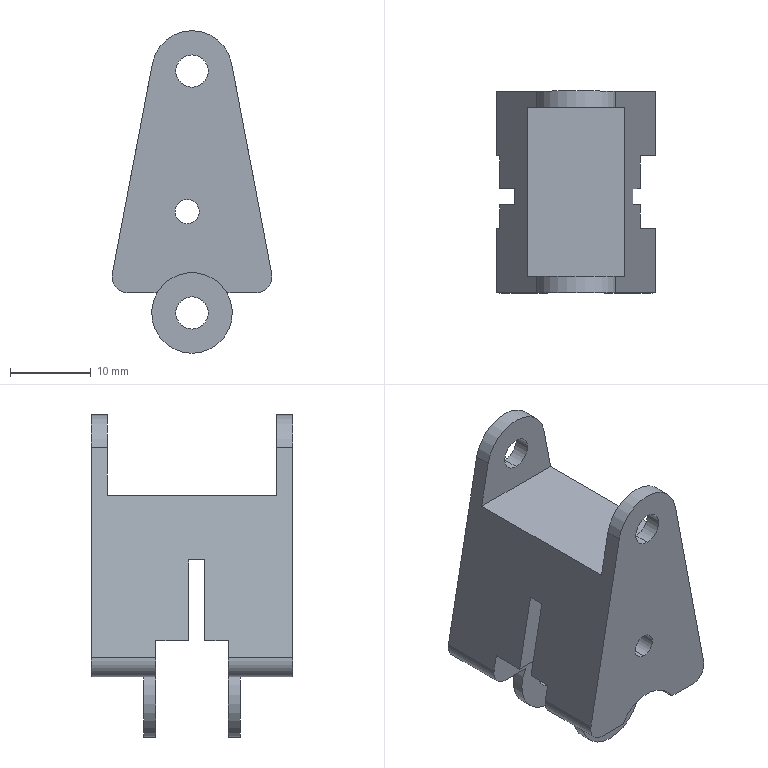Part | SolidWorks | features ICE 6, Fillet 2, Cut 1, Extrusion 1 | 1 solid | 49 faces | box 19.826 x 25 x 40 mm | volume 7993 mm3 | cylinder 25 | plane 24 | commonest cylinder face diameters 4 x12 10 x9 3 x4
STEP:
#1=CARTESIAN_POINT('',(-0.6044,12.917,14.059));
#2=VERTEX_POINT('',#1);
#3=CARTESIAN_POINT('',(-0.6044,12.917,11.059));
#4=VERTEX_POINT('',#3);
#5=CARTESIAN_POINT('',(-0.6044,12.917,12.559));
#6=DIRECTION('',(0.,-1.,0.));
#7=DIRECTION('',(0.,0.,1.));
#8=AXIS2_PLACEMENT_3D('',#5,#6,#7);
#9=CIRCLE('',#8,1.5);
#10=EDGE_CURVE('',#2,#4,#9,.T.);
#11=ORIENTED_EDGE('',*,*,#10,.T.);
#12=CARTESIAN_POINT('',(-0.6044,25.,11.059));
#13=VERTEX_POINT('',#12);
#14=CARTESIAN_POINT('',(-0.6044,0.,11.059));
#15=DIRECTION('',(0.,1.,0.));
#16=VECTOR('',#15,1000.);
#17=LINE('',#14,#16);
#18=EDGE_CURVE('',#4,#13,#17,.T.);
#19=ORIENTED_EDGE('',*,*,#18,.T.);
#20=CARTESIAN_POINT('',(-0.6044,25.,14.059));
#21=VERTEX_POINT('',#20);
#22=CARTESIAN_POINT('',(-0.6044,25.,12.559));
#23=DIRECTION('',(0.,1.,0.));
#24=DIRECTION('',(0.,0.,1.));
#25=AXIS2_PLACEMENT_3D('',#22,#23,#24);
#26=CIRCLE('',#25,1.5);
#27=EDGE_CURVE('',#13,#21,#26,.T.);
#28=ORIENTED_EDGE('',*,*,#27,.T.);
#29=CARTESIAN_POINT('',(-0.6044,0.,14.059));
#30=DIRECTION('',(0.,1.,0.));
#31=VECTOR('',#30,1000.);
#32=LINE('',#29,#31);
#33=EDGE_CURVE('',#2,#21,#32,.T.);
#34=ORIENTED_EDGE('',*,*,#33,.F.);
#35=EDGE_LOOP('',(#11,#19,#28,#34));
#36=FACE_OUTER_BOUND('',#35,.T.);
#37=CARTESIAN_POINT('',(-0.6044,0.,12.559));
#38=DIRECTION('',(0.,1.,0.));
#39=DIRECTION('',(0.,0.,1.));
#40=AXIS2_PLACEMENT_3D('',#37,#38,#39);
#41=CYLINDRICAL_SURFACE('',#40,1.5);
#42=ADVANCED_FACE('',(#36),#41,.F.);
#43=CARTESIAN_POINT('',(0.,18.5,5.));
#44=VERTEX_POINT('',#43);
#45=CARTESIAN_POINT('',(4.33,18.5,2.5));
#46=VERTEX_POINT('',#45);
#47=CARTESIAN_POINT('',(0.,18.5,0.));
#48=DIRECTION('',(0.,1.,0.));
#49=DIRECTION('',(0.,0.,1.));
#50=AXIS2_PLACEMENT_3D('',#47,#48,#49);
#51=CIRCLE('',#50,5.);
#52=EDGE_CURVE('',#44,#46,#51,.T.);
#53=ORIENTED_EDGE('',*,*,#52,.F.);
#54=CARTESIAN_POINT('',(0.,25.,5.));
#55=VERTEX_POINT('',#54);
#56=CARTESIAN_POINT('',(0.,18.5,5.));
#57=DIRECTION('',(0.,1.,0.));
#58=VECTOR('',#57,1000.);
#59=LINE('',#56,#58);
#60=EDGE_CURVE('',#44,#55,#59,.T.);
#61=ORIENTED_EDGE('',*,*,#60,.T.);
#62=CARTESIAN_POINT('',(4.33,25.,2.5));
#63=VERTEX_POINT('',#62);
#64=CARTESIAN_POINT('',(0.,25.,0.));
#65=DIRECTION('',(0.,1.,0.));
#66=DIRECTION('',(0.,0.,1.));
#67=AXIS2_PLACEMENT_3D('',#64,#65,#66);
#68=CIRCLE('',#67,5.);
#69=EDGE_CURVE('',#55,#63,#68,.T.);
#70=ORIENTED_EDGE('',*,*,#69,.T.);
#71=CARTESIAN_POINT('',(4.33,25.,2.5));
#72=DIRECTION('',(0.,-1.,0.));
#73=VECTOR('',#72,1000.);
#74=LINE('',#71,#73);
#75=EDGE_CURVE('',#63,#46,#74,.T.);
#76=ORIENTED_EDGE('',*,*,#75,.T.);
#77=EDGE_LOOP('',(#53,#61,#70,#76));
#78=FACE_OUTER_BOUND('',#77,.T.);
#79=CARTESIAN_POINT('',(0.,18.5,0.));
#80=DIRECTION('',(0.,1.,0.));
#81=DIRECTION('',(0.,0.,1.));
#82=AXIS2_PLACEMENT_3D('',#79,#80,#81);
#83=CYLINDRICAL_SURFACE('',#82,5.);
#84=ADVANCED_FACE('',(#78),#83,.F.);
#85=CARTESIAN_POINT('',(0.,0.,28.));
#86=VERTEX_POINT('',#85);
#87=CARTESIAN_POINT('',(0.,0.,32.));
#88=VERTEX_POINT('',#87);
#89=CARTESIAN_POINT('',(0.,0.,30.));
#90=DIRECTION('',(0.,1.,0.));
#91=DIRECTION('',(0.,0.,1.));
#92=AXIS2_PLACEMENT_3D('',#89,#90,#91);
#93=CIRCLE('',#92,2.);
#94=EDGE_CURVE('',#86,#88,#93,.T.);
#95=ORIENTED_EDGE('',*,*,#94,.F.);
#96=CARTESIAN_POINT('',(0.,2.,28.));
#97=VERTEX_POINT('',#96);
#98=CARTESIAN_POINT('',(0.,0.,28.));
#99=DIRECTION('',(0.,1.,0.));
#100=VECTOR('',#99,1000.);
#101=LINE('',#98,#100);
#102=EDGE_CURVE('',#86,#97,#101,.T.);
#103=ORIENTED_EDGE('',*,*,#102,.T.);
#104=CARTESIAN_POINT('',(0.,2.,32.));
#105=VERTEX_POINT('',#104);
#106=CARTESIAN_POINT('',(0.,2.,30.));
#107=DIRECTION('',(0.,1.,0.));
#108=DIRECTION('',(0.,0.,-1.));
#109=AXIS2_PLACEMENT_3D('',#106,#107,#108);
#110=CIRCLE('',#109,2.);
#111=EDGE_CURVE('',#97,#105,#110,.T.);
#112=ORIENTED_EDGE('',*,*,#111,.T.);
#113=CARTESIAN_POINT('',(0.,0.,32.));
#114=DIRECTION('',(0.,1.,0.));
#115=VECTOR('',#114,1000.);
#116=LINE('',#113,#115);
#117=EDGE_CURVE('',#88,#105,#116,.T.);
#118=ORIENTED_EDGE('',*,*,#117,.F.);
#119=EDGE_LOOP('',(#95,#103,#112,#118));
#120=FACE_OUTER_BOUND('',#119,.T.);
#121=CARTESIAN_POINT('',(0.,0.,30.));
#122=DIRECTION('',(0.,1.,0.));
#123=DIRECTION('',(0.,0.,1.));
#124=AXIS2_PLACEMENT_3D('',#121,#122,#123);
#125=CYLINDRICAL_SURFACE('',#124,2.);
#126=ADVANCED_FACE('',(#120),#125,.F.);
#127=CARTESIAN_POINT('',(0.,6.5,-2.));
#128=VERTEX_POINT('',#127);
#129=CARTESIAN_POINT('',(0.,6.5,2.));
#130=VERTEX_POINT('',#129);
#131=CARTESIAN_POINT('',(0.,6.5,0.));
#132=DIRECTION('',(0.,1.,0.));
#133=DIRECTION('',(0.,0.,-1.));
#134=AXIS2_PLACEMENT_3D('',#131,#132,#133);
#135=CIRCLE('',#134,2.);
#136=EDGE_CURVE('',#128,#130,#135,.T.);
#137=ORIENTED_EDGE('',*,*,#136,.F.);
#138=CARTESIAN_POINT('',(0.,8.,-2.));
#139=VERTEX_POINT('',#138);
#140=CARTESIAN_POINT('',(0.,0.,-2.));
#141=DIRECTION('',(0.,1.,0.));
#142=VECTOR('',#141,1000.);
#143=LINE('',#140,#142);
#144=EDGE_CURVE('',#128,#139,#143,.T.);
#145=ORIENTED_EDGE('',*,*,#144,.T.);
#146=CARTESIAN_POINT('',(0.,8.,2.));
#147=VERTEX_POINT('',#146);
#148=CARTESIAN_POINT('',(0.,8.,0.));
#149=DIRECTION('',(0.,1.,0.));
#150=DIRECTION('',(0.,0.,-1.));
#151=AXIS2_PLACEMENT_3D('',#148,#149,#150);
#152=CIRCLE('',#151,2.);
#153=EDGE_CURVE('',#139,#147,#152,.T.);
#154=ORIENTED_EDGE('',*,*,#153,.T.);
#155=CARTESIAN_POINT('',(0.,0.,2.));
#156=DIRECTION('',(0.,1.,0.));
#157=VECTOR('',#156,1000.);
#158=LINE('',#155,#157);
#159=EDGE_CURVE('',#130,#147,#158,.T.);
#160=ORIENTED_EDGE('',*,*,#159,.F.);
#161=EDGE_LOOP('',(#137,#145,#154,#160));
#162=FACE_OUTER_BOUND('',#161,.T.);
#163=CARTESIAN_POINT('',(0.,0.,0.));
#164=DIRECTION('',(0.,1.,0.));
#165=DIRECTION('',(0.,0.,1.));
#166=AXIS2_PLACEMENT_3D('',#163,#164,#165);
#167=CYLINDRICAL_SURFACE('',#166,2.);
#168=ADVANCED_FACE('',(#162),#167,.F.);
#169=CARTESIAN_POINT('',(-4.33,8.,2.5));
#170=VERTEX_POINT('',#169);
#171=CARTESIAN_POINT('',(0.,8.,-5.));
#172=VERTEX_POINT('',#171);
#173=CARTESIAN_POINT('',(0.,8.,0.));
#174=DIRECTION('',(0.,-1.,0.));
#175=DIRECTION('',(0.,0.,-1.));
#176=AXIS2_PLACEMENT_3D('',#173,#174,#175);
#177=CIRCLE('',#176,5.);
#178=EDGE_CURVE('',#170,#172,#177,.T.);
#179=ORIENTED_EDGE('',*,*,#178,.T.);
#180=CARTESIAN_POINT('',(0.,6.5,-5.));
#181=VERTEX_POINT('',#180);
#182=CARTESIAN_POINT('',(0.,25.,-5.));
#183=DIRECTION('',(0.,-1.,0.));
#184=VECTOR('',#183,1000.);
#185=LINE('',#182,#184);
#186=EDGE_CURVE('',#172,#181,#185,.T.);
#187=ORIENTED_EDGE('',*,*,#186,.T.);
#188=CARTESIAN_POINT('',(-4.33,6.5,2.5));
#189=VERTEX_POINT('',#188);
#190=CARTESIAN_POINT('',(0.,6.5,0.));
#191=DIRECTION('',(0.,-1.,0.));
#192=DIRECTION('',(0.,0.,-1.));
#193=AXIS2_PLACEMENT_3D('',#190,#191,#192);
#194=CIRCLE('',#193,5.);
#195=EDGE_CURVE('',#189,#181,#194,.T.);
#196=ORIENTED_EDGE('',*,*,#195,.F.);
#197=CARTESIAN_POINT('',(-4.33,25.,2.5));
#198=DIRECTION('',(0.,-1.,0.));
#199=VECTOR('',#198,1000.);
#200=LINE('',#197,#199);
#201=EDGE_CURVE('',#170,#189,#200,.T.);
#202=ORIENTED_EDGE('',*,*,#201,.F.);
#203=EDGE_LOOP('',(#179,#187,#196,#202));
#204=FACE_OUTER_BOUND('',#203,.T.);
#205=CARTESIAN_POINT('',(0.,25.,0.));
#206=DIRECTION('',(0.,-1.,0.));
#207=DIRECTION('',(0.,0.,-1.));
#208=AXIS2_PLACEMENT_3D('',#205,#206,#207);
#209=CYLINDRICAL_SURFACE('',#208,5.);
#210=ADVANCED_FACE('',(#204),#209,.T.);
#211=CARTESIAN_POINT('',(0.,23.,32.));
#212=VERTEX_POINT('',#211);
#213=CARTESIAN_POINT('',(0.,23.,28.));
#214=VERTEX_POINT('',#213);
#215=CARTESIAN_POINT('',(0.,23.,30.));
#216=DIRECTION('',(0.,-1.,0.));
#217=DIRECTION('',(0.,0.,1.));
#218=AXIS2_PLACEMENT_3D('',#215,#216,#217);
#219=CIRCLE('',#218,2.);
#220=EDGE_CURVE('',#212,#214,#219,.T.);
#221=ORIENTED_EDGE('',*,*,#220,.T.);
#222=CARTESIAN_POINT('',(0.,25.,28.));
#223=VERTEX_POINT('',#222);
#224=CARTESIAN_POINT('',(0.,0.,28.));
#225=DIRECTION('',(0.,1.,0.));
#226=VECTOR('',#225,1000.);
#227=LINE('',#224,#226);
#228=EDGE_CURVE('',#214,#223,#227,.T.);
#229=ORIENTED_EDGE('',*,*,#228,.T.);
#230=CARTESIAN_POINT('',(0.,25.,32.));
#231=VERTEX_POINT('',#230);
#232=CARTESIAN_POINT('',(0.,25.,30.));
#233=DIRECTION('',(0.,1.,0.));
#234=DIRECTION('',(0.,0.,1.));
#235=AXIS2_PLACEMENT_3D('',#232,#233,#234);
#236=CIRCLE('',#235,2.);
#237=EDGE_CURVE('',#223,#231,#236,.T.);
#238=ORIENTED_EDGE('',*,*,#237,.T.);
#239=CARTESIAN_POINT('',(0.,0.,32.));
#240=DIRECTION('',(0.,1.,0.));
#241=VECTOR('',#240,1000.);
#242=LINE('',#239,#241);
#243=EDGE_CURVE('',#212,#231,#242,.T.);
#244=ORIENTED_EDGE('',*,*,#243,.F.);
#245=EDGE_LOOP('',(#221,#229,#238,#244));
#246=FACE_OUTER_BOUND('',#245,.T.);
#247=CARTESIAN_POINT('',(0.,0.,30.));
#248=DIRECTION('',(0.,1.,0.));
#249=DIRECTION('',(0.,0.,1.));
#250=AXIS2_PLACEMENT_3D('',#247,#248,#249);
#251=CYLINDRICAL_SURFACE('',#250,2.);
#252=ADVANCED_FACE('',(#246),#251,.F.);
#253=CARTESIAN_POINT('',(0.,17.,2.));
#254=VERTEX_POINT('',#253);
#255=CARTESIAN_POINT('',(0.,17.,-2.));
#256=VERTEX_POINT('',#255);
#257=CARTESIAN_POINT('',(0.,17.,0.));
#258=DIRECTION('',(0.,-1.,0.));
#259=DIRECTION('',(0.,0.,1.));
#260=AXIS2_PLACEMENT_3D('',#257,#258,#259);
#261=CIRCLE('',#260,2.);
#262=EDGE_CURVE('',#254,#256,#261,.T.);
#263=ORIENTED_EDGE('',*,*,#262,.T.);
#264=CARTESIAN_POINT('',(0.,18.5,-2.));
#265=VERTEX_POINT('',#264);
#266=CARTESIAN_POINT('',(0.,0.,-2.));
#267=DIRECTION('',(0.,1.,0.));
#268=VECTOR('',#267,1000.);
#269=LINE('',#266,#268);
#270=EDGE_CURVE('',#256,#265,#269,.T.);
#271=ORIENTED_EDGE('',*,*,#270,.T.);
#272=CARTESIAN_POINT('',(0.,18.5,2.));
#273=VERTEX_POINT('',#272);
#274=CARTESIAN_POINT('',(0.,18.5,0.));
#275=DIRECTION('',(0.,-1.,0.));
#276=DIRECTION('',(0.,0.,1.));
#277=AXIS2_PLACEMENT_3D('',#274,#275,#276);
#278=CIRCLE('',#277,2.);
#279=EDGE_CURVE('',#273,#265,#278,.T.);
#280=ORIENTED_EDGE('',*,*,#279,.F.);
#281=CARTESIAN_POINT('',(0.,0.,2.));
#282=DIRECTION('',(0.,1.,0.));
#283=VECTOR('',#282,1000.);
#284=LINE('',#281,#283);
#285=EDGE_CURVE('',#254,#273,#284,.T.);
#286=ORIENTED_EDGE('',*,*,#285,.F.);
#287=EDGE_LOOP('',(#263,#271,#280,#286));
#288=FACE_OUTER_BOUND('',#287,.T.);
#289=CARTESIAN_POINT('',(0.,0.,0.));
#290=DIRECTION('',(0.,1.,0.));
#291=DIRECTION('',(0.,0.,1.));
#292=AXIS2_PLACEMENT_3D('',#289,#290,#291);
#293=CYLINDRICAL_SURFACE('',#292,2.);
#294=ADVANCED_FACE('',(#288),#293,.F.);
#295=CARTESIAN_POINT('',(0.,18.5,-5.));
#296=VERTEX_POINT('',#295);
#297=CARTESIAN_POINT('',(-4.33,18.5,2.5));
#298=VERTEX_POINT('',#297);
#299=CARTESIAN_POINT('',(0.,18.5,0.));
#300=DIRECTION('',(0.,1.,0.));
#301=DIRECTION('',(0.,0.,1.));
#302=AXIS2_PLACEMENT_3D('',#299,#300,#301);
#303=CIRCLE('',#302,5.);
#304=EDGE_CURVE('',#296,#298,#303,.T.);
#305=ORIENTED_EDGE('',*,*,#304,.F.);
#306=CARTESIAN_POINT('',(0.,17.,-5.));
#307=VERTEX_POINT('',#306);
#308=CARTESIAN_POINT('',(0.,25.,-5.));
#309=DIRECTION('',(0.,-1.,0.));
#310=VECTOR('',#309,1000.);
#311=LINE('',#308,#310);
#312=EDGE_CURVE('',#296,#307,#311,.T.);
#313=ORIENTED_EDGE('',*,*,#312,.T.);
#314=CARTESIAN_POINT('',(-4.33,17.,2.5));
#315=VERTEX_POINT('',#314);
#316=CARTESIAN_POINT('',(0.,17.,0.));
#317=DIRECTION('',(0.,1.,0.));
#318=DIRECTION('',(0.,0.,1.));
#319=AXIS2_PLACEMENT_3D('',#316,#317,#318);
#320=CIRCLE('',#319,5.);
#321=EDGE_CURVE('',#307,#315,#320,.T.);
#322=ORIENTED_EDGE('',*,*,#321,.T.);
#323=CARTESIAN_POINT('',(-4.33,25.,2.5));
#324=DIRECTION('',(0.,-1.,0.));
#325=VECTOR('',#324,1000.);
#326=LINE('',#323,#325);
#327=EDGE_CURVE('',#298,#315,#326,.T.);
#328=ORIENTED_EDGE('',*,*,#327,.F.);
#329=EDGE_LOOP('',(#305,#313,#322,#328));
#330=FACE_OUTER_BOUND('',#329,.T.);
#331=CARTESIAN_POINT('',(0.,25.,0.));
#332=DIRECTION('',(0.,-1.,0.));
#333=DIRECTION('',(0.,0.,-1.));
#334=AXIS2_PLACEMENT_3D('',#331,#332,#333);
#335=CYLINDRICAL_SURFACE('',#334,5.);
#336=ADVANCED_FACE('',(#330),#335,.T.);
#337=CARTESIAN_POINT('',(-0.6044,0.,11.059));
#338=VERTEX_POINT('',#337);
#339=CARTESIAN_POINT('',(-0.6044,0.,14.059));
#340=VERTEX_POINT('',#339);
#341=CARTESIAN_POINT('',(-0.6044,0.,12.559));
#342=DIRECTION('',(0.,1.,0.));
#343=DIRECTION('',(0.,0.,1.));
#344=AXIS2_PLACEMENT_3D('',#341,#342,#343);
#345=CIRCLE('',#344,1.5);
#346=EDGE_CURVE('',#338,#340,#345,.T.);
#347=ORIENTED_EDGE('',*,*,#346,.F.);
#348=CARTESIAN_POINT('',(-0.6044,10.917,11.059));
#349=VERTEX_POINT('',#348);
#350=CARTESIAN_POINT('',(-0.6044,0.,11.059));
#351=DIRECTION('',(0.,1.,0.));
#352=VECTOR('',#351,1000.);
#353=LINE('',#350,#352);
#354=EDGE_CURVE('',#338,#349,#353,.T.);
#355=ORIENTED_EDGE('',*,*,#354,.T.);
#356=CARTESIAN_POINT('',(-0.6044,10.917,14.059));
#357=VERTEX_POINT('',#356);
#358=CARTESIAN_POINT('',(-0.6044,10.917,12.559));
#359=DIRECTION('',(0.,1.,0.));
#360=DIRECTION('',(0.,0.,-1.));
#361=AXIS2_PLACEMENT_3D('',#358,#359,#360);
#362=CIRCLE('',#361,1.5);
#363=EDGE_CURVE('',#349,#357,#362,.T.);
#364=ORIENTED_EDGE('',*,*,#363,.T.);
#365=CARTESIAN_POINT('',(-0.6044,0.,14.059));
#366=DIRECTION('',(0.,1.,0.));
#367=VECTOR('',#366,1000.);
#368=LINE('',#365,#367);
#369=EDGE_CURVE('',#340,#357,#368,.T.);
#370=ORIENTED_EDGE('',*,*,#369,.F.);
#371=EDGE_LOOP('',(#347,#355,#364,#370));
#372=FACE_OUTER_BOUND('',#371,.T.);
#373=CARTESIAN_POINT('',(-0.6044,0.,12.559));
#374=DIRECTION('',(0.,1.,0.));
#375=DIRECTION('',(0.,0.,1.));
#376=AXIS2_PLACEMENT_3D('',#373,#374,#375);
#377=CYLINDRICAL_SURFACE('',#376,1.5);
#378=ADVANCED_FACE('',(#372),#377,.F.);
#379=CARTESIAN_POINT('',(-9.473,10.917,7.));
#380=VERTEX_POINT('',#379);
#381=CARTESIAN_POINT('',(-9.473,8.,7.));
#382=VERTEX_POINT('',#381);
#383=CARTESIAN_POINT('',(-9.473,25.,7.));
#384=DIRECTION('',(0.,-1.,0.));
#385=VECTOR('',#384,1000.);
#386=LINE('',#383,#385);
#387=EDGE_CURVE('',#380,#382,#386,.T.);
#388=ORIENTED_EDGE('',*,*,#387,.F.);
#389=CARTESIAN_POINT('',(7.437,10.917,7.));
#390=VERTEX_POINT('',#389);
#391=CARTESIAN_POINT('',(-9.913,10.917,7.));
#392=DIRECTION('',(1.,0.,0.));
#393=VECTOR('',#392,1000.);
#394=LINE('',#391,#393);
#395=EDGE_CURVE('',#380,#390,#394,.T.);
#396=ORIENTED_EDGE('',*,*,#395,.T.);
#397=CARTESIAN_POINT('',(7.437,8.,7.));
#398=VERTEX_POINT('',#397);
#399=CARTESIAN_POINT('',(7.437,8.,7.));
#400=DIRECTION('',(0.,-1.,0.));
#401=VECTOR('',#400,1000.);
#402=LINE('',#399,#401);
#403=EDGE_CURVE('',#390,#398,#402,.T.);
#404=ORIENTED_EDGE('',*,*,#403,.T.);
#405=CARTESIAN_POINT('',(-9.913,8.,7.));
#406=DIRECTION('',(1.,0.,0.));
#407=VECTOR('',#406,1000.);
#408=LINE('',#405,#407);
#409=EDGE_CURVE('',#382,#398,#408,.T.);
#410=ORIENTED_EDGE('',*,*,#409,.F.);
#411=EDGE_LOOP('',(#388,#396,#404,#410));
#412=FACE_OUTER_BOUND('',#411,.T.);
#413=CARTESIAN_POINT('',(-9.913,8.,7.));
#414=DIRECTION('',(0.,0.,1.));
#415=DIRECTION('',(1.,0.,0.));
#416=AXIS2_PLACEMENT_3D('',#413,#414,#415);
#417=PLANE('',#416);
#418=ADVANCED_FACE('',(#412),#417,.F.);
#419=ORIENTED_EDGE('',*,*,#403,.F.);
#420=CARTESIAN_POINT('',(6.011,10.917,14.484));
#421=VERTEX_POINT('',#420);
#422=CARTESIAN_POINT('',(8.463,10.917,1.613));
#423=DIRECTION('',(-0.1872,0.,0.9823));
#424=VECTOR('',#423,1000.);
#425=LINE('',#422,#424);
#426=EDGE_CURVE('',#390,#421,#425,.T.);
#427=ORIENTED_EDGE('',*,*,#426,.T.);
#428=CARTESIAN_POINT('',(6.011,8.,14.484));
#429=VERTEX_POINT('',#428);
#430=CARTESIAN_POINT('',(6.011,8.,14.484));
#431=DIRECTION('',(0.,-1.,0.));
#432=VECTOR('',#431,1000.);
#433=LINE('',#430,#432);
#434=EDGE_CURVE('',#421,#429,#433,.T.);
#435=ORIENTED_EDGE('',*,*,#434,.T.);
#436=CARTESIAN_POINT('',(7.508,8.,6.626));
#437=DIRECTION('',(0.1872,0.,-0.9823));
#438=VECTOR('',#437,1000.);
#439=LINE('',#436,#438);
#440=EDGE_CURVE('',#429,#398,#439,.T.);
#441=ORIENTED_EDGE('',*,*,#440,.T.);
#442=EDGE_LOOP('',(#419,#427,#435,#441));
#443=FACE_OUTER_BOUND('',#442,.T.);
#444=CARTESIAN_POINT('',(8.463,0.,1.613));
#445=DIRECTION('',(-0.9823,0.,-0.1872));
#446=DIRECTION('',(-0.1872,0.,0.9823));
#447=AXIS2_PLACEMENT_3D('',#444,#445,#446);
#448=PLANE('',#447);
#449=ADVANCED_FACE('',(#443),#448,.F.);
#450=ORIENTED_EDGE('',*,*,#434,.F.);
#451=CARTESIAN_POINT('',(7.975,10.917,14.859));
#452=VERTEX_POINT('',#451);
#453=CARTESIAN_POINT('',(6.011,10.917,14.484));
#454=DIRECTION('',(0.9823,0.,0.1872));
#455=VECTOR('',#454,1000.);
#456=LINE('',#453,#455);
#457=EDGE_CURVE('',#421,#452,#456,.T.);
#458=ORIENTED_EDGE('',*,*,#457,.T.);
#459=CARTESIAN_POINT('',(7.975,8.,14.859));
#460=VERTEX_POINT('',#459);
#461=CARTESIAN_POINT('',(7.975,8.,14.859));
#462=DIRECTION('',(0.,-1.,0.));
#463=VECTOR('',#462,1000.);
#464=LINE('',#461,#463);
#465=EDGE_CURVE('',#452,#460,#464,.T.);
#466=ORIENTED_EDGE('',*,*,#465,.T.);
#467=CARTESIAN_POINT('',(6.011,8.,14.484));
#468=DIRECTION('',(0.9823,0.,0.1872));
#469=VECTOR('',#468,1000.);
#470=LINE('',#467,#469);
#471=EDGE_CURVE('',#429,#460,#470,.T.);
#472=ORIENTED_EDGE('',*,*,#471,.F.);
#473=EDGE_LOOP('',(#450,#458,#466,#472));
#474=FACE_OUTER_BOUND('',#473,.T.);
#475=CARTESIAN_POINT('',(6.011,8.,14.484));
#476=DIRECTION('',(-0.1872,0.,0.9823));
#477=DIRECTION('',(0.9823,0.,0.1872));
#478=AXIS2_PLACEMENT_3D('',#475,#476,#477);
#479=PLANE('',#478);
#480=ADVANCED_FACE('',(#474),#479,.F.);
#481=ORIENTED_EDGE('',*,*,#354,.F.);
#482=CARTESIAN_POINT('',(-0.6044,0.,12.559));
#483=DIRECTION('',(0.,1.,0.));
#484=DIRECTION('',(0.,0.,1.));
#485=AXIS2_PLACEMENT_3D('',#482,#483,#484);
#486=CIRCLE('',#485,1.5);
#487=EDGE_CURVE('',#340,#338,#486,.T.);
#488=ORIENTED_EDGE('',*,*,#487,.F.);
#489=ORIENTED_EDGE('',*,*,#369,.T.);
#490=CARTESIAN_POINT('',(-0.6044,10.917,12.559));
#491=DIRECTION('',(0.,1.,0.));
#492=DIRECTION('',(0.,0.,-1.));
#493=AXIS2_PLACEMENT_3D('',#490,#491,#492);
#494=CIRCLE('',#493,1.5);
#495=EDGE_CURVE('',#357,#349,#494,.T.);
#496=ORIENTED_EDGE('',*,*,#495,.T.);
#497=EDGE_LOOP('',(#481,#488,#489,#496));
#498=FACE_OUTER_BOUND('',#497,.T.);
#499=CARTESIAN_POINT('',(-0.6044,0.,12.559));
#500=DIRECTION('',(0.,1.,0.));
#501=DIRECTION('',(0.,0.,1.));
#502=AXIS2_PLACEMENT_3D('',#499,#500,#501);
#503=CYLINDRICAL_SURFACE('',#502,1.5);
#504=ADVANCED_FACE('',(#498),#503,.F.);
#505=ORIENTED_EDGE('',*,*,#312,.F.);
#506=CARTESIAN_POINT('',(0.,18.5,0.));
#507=DIRECTION('',(0.,1.,0.));
#508=DIRECTION('',(0.,0.,1.));
#509=AXIS2_PLACEMENT_3D('',#506,#507,#508);
#510=CIRCLE('',#509,5.);
#511=EDGE_CURVE('',#46,#296,#510,.T.);
#512=ORIENTED_EDGE('',*,*,#511,.F.);
#513=CARTESIAN_POINT('',(4.33,17.,2.5));
#514=VERTEX_POINT('',#513);
#515=CARTESIAN_POINT('',(4.33,25.,2.5));
#516=DIRECTION('',(0.,-1.,0.));
#517=VECTOR('',#516,1000.);
#518=LINE('',#515,#517);
#519=EDGE_CURVE('',#46,#514,#518,.T.);
#520=ORIENTED_EDGE('',*,*,#519,.T.);
#521=CARTESIAN_POINT('',(0.,17.,0.));
#522=DIRECTION('',(0.,1.,0.));
#523=DIRECTION('',(0.,0.,1.));
#524=AXIS2_PLACEMENT_3D('',#521,#522,#523);
#525=CIRCLE('',#524,5.);
#526=EDGE_CURVE('',#514,#307,#525,.T.);
#527=ORIENTED_EDGE('',*,*,#526,.T.);
#528=EDGE_LOOP('',(#505,#512,#520,#527));
#529=FACE_OUTER_BOUND('',#528,.T.);
#530=CARTESIAN_POINT('',(0.,25.,0.));
#531=DIRECTION('',(0.,-1.,0.));
#532=DIRECTION('',(0.,0.,-1.));
#533=AXIS2_PLACEMENT_3D('',#530,#531,#532);
#534=CYLINDRICAL_SURFACE('',#533,5.);
#535=ADVANCED_FACE('',(#529),#534,.T.);
#536=ORIENTED_EDGE('',*,*,#270,.F.);
#537=CARTESIAN_POINT('',(0.,17.,0.));
#538=DIRECTION('',(0.,-1.,0.));
#539=DIRECTION('',(0.,0.,1.));
#540=AXIS2_PLACEMENT_3D('',#537,#538,#539);
#541=CIRCLE('',#540,2.);
#542=EDGE_CURVE('',#256,#254,#541,.T.);
#543=ORIENTED_EDGE('',*,*,#542,.T.);
#544=ORIENTED_EDGE('',*,*,#285,.T.);
#545=CARTESIAN_POINT('',(0.,18.5,0.));
#546=DIRECTION('',(0.,-1.,0.));
#547=DIRECTION('',(0.,0.,1.));
#548=AXIS2_PLACEMENT_3D('',#545,#546,#547);
#549=CIRCLE('',#548,2.);
#550=EDGE_CURVE('',#265,#273,#549,.T.);
#551=ORIENTED_EDGE('',*,*,#550,.F.);
#552=EDGE_LOOP('',(#536,#543,#544,#551));
#553=FACE_OUTER_BOUND('',#552,.T.);
#554=CARTESIAN_POINT('',(0.,0.,0.));
#555=DIRECTION('',(0.,1.,0.));
#556=DIRECTION('',(0.,0.,1.));
#557=AXIS2_PLACEMENT_3D('',#554,#555,#556);
#558=CYLINDRICAL_SURFACE('',#557,2.);
#559=ADVANCED_FACE('',(#553),#558,.F.);
#560=ORIENTED_EDGE('',*,*,#327,.T.);
#561=CARTESIAN_POINT('',(-7.913,17.,2.5));
#562=VERTEX_POINT('',#561);
#563=CARTESIAN_POINT('',(-4.33,17.,2.5));
#564=DIRECTION('',(-1.,0.,0.));
#565=VECTOR('',#564,1000.);
#566=LINE('',#563,#565);
#567=EDGE_CURVE('',#315,#562,#566,.T.);
#568=ORIENTED_EDGE('',*,*,#567,.T.);
#569=CARTESIAN_POINT('',(-7.913,25.,2.5));
#570=VERTEX_POINT('',#569);
#571=CARTESIAN_POINT('',(-7.913,25.,2.5));
#572=DIRECTION('',(0.,1.,0.));
#573=VECTOR('',#572,1000.);
#574=LINE('',#571,#573);
#575=EDGE_CURVE('',#562,#570,#574,.T.);
#576=ORIENTED_EDGE('',*,*,#575,.T.);
#577=CARTESIAN_POINT('',(-4.33,25.,2.5));
#578=VERTEX_POINT('',#577);
#579=CARTESIAN_POINT('',(-4.33,25.,2.5));
#580=DIRECTION('',(-1.,0.,0.));
#581=VECTOR('',#580,1000.);
#582=LINE('',#579,#581);
#583=EDGE_CURVE('',#578,#570,#582,.T.);
#584=ORIENTED_EDGE('',*,*,#583,.F.);
#585=CARTESIAN_POINT('',(-4.33,25.,2.5));
#586=DIRECTION('',(0.,-1.,0.));
#587=VECTOR('',#586,1000.);
#588=LINE('',#585,#587);
#589=EDGE_CURVE('',#578,#298,#588,.T.);
#590=ORIENTED_EDGE('',*,*,#589,.T.);
#591=EDGE_LOOP('',(#560,#568,#576,#584,#590));
#592=FACE_OUTER_BOUND('',#591,.T.);
#593=CARTESIAN_POINT('',(-4.33,25.,2.5));
#594=DIRECTION('',(0.,0.,1.));
#595=DIRECTION('',(1.,0.,0.));
#596=AXIS2_PLACEMENT_3D('',#593,#594,#595);
#597=PLANE('',#596);
#598=ADVANCED_FACE('',(#592),#597,.F.);
#599=CARTESIAN_POINT('',(-4.912,23.,30.936));
#600=VERTEX_POINT('',#599);
#601=CARTESIAN_POINT('',(4.912,23.,30.936));
#602=VERTEX_POINT('',#601);
#603=CARTESIAN_POINT('',(0.,23.,30.));
#604=DIRECTION('',(0.,1.,0.));
#605=DIRECTION('',(0.,0.,1.));
#606=AXIS2_PLACEMENT_3D('',#603,#604,#605);
#607=CIRCLE('',#606,5.);
#608=EDGE_CURVE('',#600,#602,#607,.T.);
#609=ORIENTED_EDGE('',*,*,#608,.T.);
#610=CARTESIAN_POINT('',(4.912,25.,30.936));
#611=VERTEX_POINT('',#610);
#612=CARTESIAN_POINT('',(4.912,25.,30.936));
#613=DIRECTION('',(0.,-1.,0.));
#614=VECTOR('',#613,1000.);
#615=LINE('',#612,#614);
#616=EDGE_CURVE('',#611,#602,#615,.T.);
#617=ORIENTED_EDGE('',*,*,#616,.F.);
#618=CARTESIAN_POINT('',(-4.912,25.,30.936));
#619=VERTEX_POINT('',#618);
#620=CARTESIAN_POINT('',(0.,25.,30.));
#621=DIRECTION('',(0.,1.,0.));
#622=DIRECTION('',(0.,0.,1.));
#623=AXIS2_PLACEMENT_3D('',#620,#621,#622);
#624=CIRCLE('',#623,5.);
#625=EDGE_CURVE('',#619,#611,#624,.T.);
#626=ORIENTED_EDGE('',*,*,#625,.F.);
#627=CARTESIAN_POINT('',(-4.912,25.,30.936));
#628=DIRECTION('',(0.,-1.,0.));
#629=VECTOR('',#628,1000.);
#630=LINE('',#627,#629);
#631=EDGE_CURVE('',#619,#600,#630,.T.);
#632=ORIENTED_EDGE('',*,*,#631,.T.);
#633=EDGE_LOOP('',(#609,#617,#626,#632));
#634=FACE_OUTER_BOUND('',#633,.T.);
#635=CARTESIAN_POINT('',(0.,25.,30.));
#636=DIRECTION('',(0.,-1.,0.));
#637=DIRECTION('',(0.,0.,-1.));
#638=AXIS2_PLACEMENT_3D('',#635,#636,#637);
#639=CYLINDRICAL_SURFACE('',#638,5.);
#640=ADVANCED_FACE('',(#634),#639,.T.);
#641=CARTESIAN_POINT('',(7.913,25.,2.5));
#642=VERTEX_POINT('',#641);
#643=CARTESIAN_POINT('',(7.913,17.,2.5));
#644=VERTEX_POINT('',#643);
#645=CARTESIAN_POINT('',(7.913,25.,2.5));
#646=DIRECTION('',(0.,-1.,0.));
#647=VECTOR('',#646,1000.);
#648=LINE('',#645,#647);
#649=EDGE_CURVE('',#642,#644,#648,.T.);
#650=ORIENTED_EDGE('',*,*,#649,.T.);
#651=CARTESIAN_POINT('',(4.33,17.,2.5));
#652=DIRECTION('',(-1.,0.,0.));
#653=VECTOR('',#652,1000.);
#654=LINE('',#651,#653);
#655=EDGE_CURVE('',#644,#514,#654,.T.);
#656=ORIENTED_EDGE('',*,*,#655,.T.);
#657=ORIENTED_EDGE('',*,*,#519,.F.);
#658=ORIENTED_EDGE('',*,*,#75,.F.);
#659=CARTESIAN_POINT('',(4.33,25.,2.5));
#660=DIRECTION('',(-1.,0.,0.));
#661=VECTOR('',#660,1000.);
#662=LINE('',#659,#661);
#663=EDGE_CURVE('',#642,#63,#662,.T.);
#664=ORIENTED_EDGE('',*,*,#663,.F.);
#665=EDGE_LOOP('',(#650,#656,#657,#658,#664));
#666=FACE_OUTER_BOUND('',#665,.T.);
#667=CARTESIAN_POINT('',(4.33,25.,2.5));
#668=DIRECTION('',(0.,0.,1.));
#669=DIRECTION('',(1.,0.,0.));
#670=AXIS2_PLACEMENT_3D('',#667,#668,#669);
#671=PLANE('',#670);
#672=ADVANCED_FACE('',(#666),#671,.F.);
#673=ORIENTED_EDGE('',*,*,#228,.F.);
#674=CARTESIAN_POINT('',(0.,23.,30.));
#675=DIRECTION('',(0.,-1.,0.));
#676=DIRECTION('',(0.,0.,1.));
#677=AXIS2_PLACEMENT_3D('',#674,#675,#676);
#678=CIRCLE('',#677,2.);
#679=EDGE_CURVE('',#214,#212,#678,.T.);
#680=ORIENTED_EDGE('',*,*,#679,.T.);
#681=ORIENTED_EDGE('',*,*,#243,.T.);
#682=CARTESIAN_POINT('',(0.,25.,30.));
#683=DIRECTION('',(0.,1.,0.));
#684=DIRECTION('',(0.,0.,1.));
#685=AXIS2_PLACEMENT_3D('',#682,#683,#684);
#686=CIRCLE('',#685,2.);
#687=EDGE_CURVE('',#231,#223,#686,.T.);
#688=ORIENTED_EDGE('',*,*,#687,.T.);
#689=EDGE_LOOP('',(#673,#680,#681,#688));
#690=FACE_OUTER_BOUND('',#689,.T.);
#691=CARTESIAN_POINT('',(0.,0.,30.));
#692=DIRECTION('',(0.,1.,0.));
#693=DIRECTION('',(0.,0.,1.));
#694=AXIS2_PLACEMENT_3D('',#691,#692,#693);
#695=CYLINDRICAL_SURFACE('',#694,2.);
#696=ADVANCED_FACE('',(#690),#695,.F.);
#697=CARTESIAN_POINT('',(9.878,8.,4.874));
#698=VERTEX_POINT('',#697);
#699=CARTESIAN_POINT('',(7.913,8.,2.5));
#700=VERTEX_POINT('',#699);
#701=CARTESIAN_POINT('',(7.913,8.,4.5));
#702=DIRECTION('',(0.,1.,0.));
#703=DIRECTION('',(0.,0.,-1.));
#704=AXIS2_PLACEMENT_3D('',#701,#702,#703);
#705=CIRCLE('',#704,2.);
#706=EDGE_CURVE('',#698,#700,#705,.T.);
#707=ORIENTED_EDGE('',*,*,#706,.F.);
#708=CARTESIAN_POINT('',(9.878,0.,4.874));
#709=VERTEX_POINT('',#708);
#710=CARTESIAN_POINT('',(9.878,25.,4.874));
#711=DIRECTION('',(0.,1.,0.));
#712=VECTOR('',#711,1000.);
#713=LINE('',#710,#712);
#714=EDGE_CURVE('',#709,#698,#713,.T.);
#715=ORIENTED_EDGE('',*,*,#714,.F.);
#716=CARTESIAN_POINT('',(7.913,0.,2.5));
#717=VERTEX_POINT('',#716);
#718=CARTESIAN_POINT('',(7.913,0.,4.5));
#719=DIRECTION('',(0.,-1.,0.));
#720=DIRECTION('',(0.,0.,1.));
#721=AXIS2_PLACEMENT_3D('',#718,#719,#720);
#722=CIRCLE('',#721,2.);
#723=EDGE_CURVE('',#717,#709,#722,.T.);
#724=ORIENTED_EDGE('',*,*,#723,.F.);
#725=CARTESIAN_POINT('',(7.913,25.,2.5));
#726=DIRECTION('',(0.,-1.,0.));
#727=VECTOR('',#726,1000.);
#728=LINE('',#725,#727);
#729=EDGE_CURVE('',#700,#717,#728,.T.);
#730=ORIENTED_EDGE('',*,*,#729,.F.);
#731=EDGE_LOOP('',(#707,#715,#724,#730));
#732=FACE_OUTER_BOUND('',#731,.T.);
#733=CARTESIAN_POINT('',(7.913,25.,4.5));
#734=DIRECTION('',(0.,-1.,0.));
#735=DIRECTION('',(0.,0.,-1.));
#736=AXIS2_PLACEMENT_3D('',#733,#734,#735);
#737=CYLINDRICAL_SURFACE('',#736,2.);
#738=ADVANCED_FACE('',(#732),#737,.T.);
#739=CARTESIAN_POINT('',(-9.878,8.,4.874));
#740=VERTEX_POINT('',#739);
#741=CARTESIAN_POINT('',(-9.878,0.,4.874));
#742=VERTEX_POINT('',#741);
#743=CARTESIAN_POINT('',(-9.878,25.,4.874));
#744=DIRECTION('',(0.,-1.,0.));
#745=VECTOR('',#744,1000.);
#746=LINE('',#743,#745);
#747=EDGE_CURVE('',#740,#742,#746,.T.);
#748=ORIENTED_EDGE('',*,*,#747,.F.);
#749=CARTESIAN_POINT('',(-7.913,8.,2.5));
#750=VERTEX_POINT('',#749);
#751=CARTESIAN_POINT('',(-7.913,8.,4.5));
#752=DIRECTION('',(0.,1.,0.));
#753=DIRECTION('',(0.,0.,-1.));
#754=AXIS2_PLACEMENT_3D('',#751,#752,#753);
#755=CIRCLE('',#754,2.);
#756=EDGE_CURVE('',#750,#740,#755,.T.);
#757=ORIENTED_EDGE('',*,*,#756,.F.);
#758=CARTESIAN_POINT('',(-7.913,0.,2.5));
#759=VERTEX_POINT('',#758);
#760=CARTESIAN_POINT('',(-7.913,25.,2.5));
#761=DIRECTION('',(0.,1.,0.));
#762=VECTOR('',#761,1000.);
#763=LINE('',#760,#762);
#764=EDGE_CURVE('',#759,#750,#763,.T.);
#765=ORIENTED_EDGE('',*,*,#764,.F.);
#766=CARTESIAN_POINT('',(-7.913,0.,4.5));
#767=DIRECTION('',(0.,-1.,0.));
#768=DIRECTION('',(0.,0.,1.));
#769=AXIS2_PLACEMENT_3D('',#766,#767,#768);
#770=CIRCLE('',#769,2.);
#771=EDGE_CURVE('',#742,#759,#770,.T.);
#772=ORIENTED_EDGE('',*,*,#771,.F.);
#773=EDGE_LOOP('',(#748,#757,#765,#772));
#774=FACE_OUTER_BOUND('',#773,.T.);
#775=CARTESIAN_POINT('',(-7.913,25.,4.5));
#776=DIRECTION('',(0.,-1.,0.));
#777=DIRECTION('',(0.,0.,-1.));
#778=AXIS2_PLACEMENT_3D('',#775,#776,#777);
#779=CYLINDRICAL_SURFACE('',#778,2.);
#780=ADVANCED_FACE('',(#774),#779,.T.);
#781=ORIENTED_EDGE('',*,*,#186,.F.);
#782=CARTESIAN_POINT('',(4.33,8.,2.5));
#783=VERTEX_POINT('',#782);
#784=CARTESIAN_POINT('',(0.,8.,0.));
#785=DIRECTION('',(0.,-1.,0.));
#786=DIRECTION('',(0.,0.,-1.));
#787=AXIS2_PLACEMENT_3D('',#784,#785,#786);
#788=CIRCLE('',#787,5.);
#789=EDGE_CURVE('',#172,#783,#788,.T.);
#790=ORIENTED_EDGE('',*,*,#789,.T.);
#791=CARTESIAN_POINT('',(4.33,6.5,2.5));
#792=VERTEX_POINT('',#791);
#793=CARTESIAN_POINT('',(4.33,25.,2.5));
#794=DIRECTION('',(0.,-1.,0.));
#795=VECTOR('',#794,1000.);
#796=LINE('',#793,#795);
#797=EDGE_CURVE('',#783,#792,#796,.T.);
#798=ORIENTED_EDGE('',*,*,#797,.T.);
#799=CARTESIAN_POINT('',(0.,6.5,0.));
#800=DIRECTION('',(0.,-1.,0.));
#801=DIRECTION('',(0.,0.,-1.));
#802=AXIS2_PLACEMENT_3D('',#799,#800,#801);
#803=CIRCLE('',#802,5.);
#804=EDGE_CURVE('',#181,#792,#803,.T.);
#805=ORIENTED_EDGE('',*,*,#804,.F.);
#806=EDGE_LOOP('',(#781,#790,#798,#805));
#807=FACE_OUTER_BOUND('',#806,.T.);
#808=CARTESIAN_POINT('',(0.,25.,0.));
#809=DIRECTION('',(0.,-1.,0.));
#810=DIRECTION('',(0.,0.,-1.));
#811=AXIS2_PLACEMENT_3D('',#808,#809,#810);
#812=CYLINDRICAL_SURFACE('',#811,5.);
#813=ADVANCED_FACE('',(#807),#812,.T.);
#814=ORIENTED_EDGE('',*,*,#144,.F.);
#815=CARTESIAN_POINT('',(0.,6.5,0.));
#816=DIRECTION('',(0.,1.,0.));
#817=DIRECTION('',(0.,0.,-1.));
#818=AXIS2_PLACEMENT_3D('',#815,#816,#817);
#819=CIRCLE('',#818,2.);
#820=EDGE_CURVE('',#130,#128,#819,.T.);
#821=ORIENTED_EDGE('',*,*,#820,.F.);
#822=ORIENTED_EDGE('',*,*,#159,.T.);
#823=CARTESIAN_POINT('',(0.,8.,0.));
#824=DIRECTION('',(0.,1.,0.));
#825=DIRECTION('',(0.,0.,-1.));
#826=AXIS2_PLACEMENT_3D('',#823,#824,#825);
#827=CIRCLE('',#826,2.);
#828=EDGE_CURVE('',#147,#139,#827,.T.);
#829=ORIENTED_EDGE('',*,*,#828,.T.);
#830=EDGE_LOOP('',(#814,#821,#822,#829));
#831=FACE_OUTER_BOUND('',#830,.T.);
#832=CARTESIAN_POINT('',(0.,0.,0.));
#833=DIRECTION('',(0.,1.,0.));
#834=DIRECTION('',(0.,0.,1.));
#835=AXIS2_PLACEMENT_3D('',#832,#833,#834);
#836=CYLINDRICAL_SURFACE('',#835,2.);
#837=ADVANCED_FACE('',(#831),#836,.F.);
#838=ORIENTED_EDGE('',*,*,#764,.T.);
#839=CARTESIAN_POINT('',(-4.33,8.,2.5));
#840=DIRECTION('',(1.,0.,0.));
#841=VECTOR('',#840,1000.);
#842=LINE('',#839,#841);
#843=EDGE_CURVE('',#750,#170,#842,.T.);
#844=ORIENTED_EDGE('',*,*,#843,.T.);
#845=ORIENTED_EDGE('',*,*,#201,.T.);
#846=CARTESIAN_POINT('',(-4.33,0.,2.5));
#847=VERTEX_POINT('',#846);
#848=CARTESIAN_POINT('',(-4.33,6.5,2.5));
#849=DIRECTION('',(0.,-1.,0.));
#850=VECTOR('',#849,1000.);
#851=LINE('',#848,#850);
#852=EDGE_CURVE('',#189,#847,#851,.T.);
#853=ORIENTED_EDGE('',*,*,#852,.T.);
#854=CARTESIAN_POINT('',(-4.33,0.,2.5));
#855=DIRECTION('',(-1.,0.,0.));
#856=VECTOR('',#855,1000.);
#857=LINE('',#854,#856);
#858=EDGE_CURVE('',#847,#759,#857,.T.);
#859=ORIENTED_EDGE('',*,*,#858,.T.);
#860=EDGE_LOOP('',(#838,#844,#845,#853,#859));
#861=FACE_OUTER_BOUND('',#860,.T.);
#862=CARTESIAN_POINT('',(-4.33,25.,2.5));
#863=DIRECTION('',(0.,0.,1.));
#864=DIRECTION('',(1.,0.,0.));
#865=AXIS2_PLACEMENT_3D('',#862,#863,#864);
#866=PLANE('',#865);
#867=ADVANCED_FACE('',(#861),#866,.F.);
#868=CARTESIAN_POINT('',(-7.57,12.917,16.987));
#869=VERTEX_POINT('',#868);
#870=CARTESIAN_POINT('',(-7.57,10.917,16.987));
#871=VERTEX_POINT('',#870);
#872=CARTESIAN_POINT('',(-7.57,25.,16.987));
#873=DIRECTION('',(0.,-1.,0.));
#874=VECTOR('',#873,1000.);
#875=LINE('',#872,#874);
#876=EDGE_CURVE('',#869,#871,#875,.T.);
#877=ORIENTED_EDGE('',*,*,#876,.T.);
#878=CARTESIAN_POINT('',(-10.33,10.917,2.5));
#879=DIRECTION('',(-0.1872,0.,-0.9823));
#880=VECTOR('',#879,1000.);
#881=LINE('',#878,#880);
#882=EDGE_CURVE('',#871,#380,#881,.T.);
#883=ORIENTED_EDGE('',*,*,#882,.T.);
#884=ORIENTED_EDGE('',*,*,#387,.T.);
#885=CARTESIAN_POINT('',(-10.33,8.,2.5));
#886=DIRECTION('',(-0.1872,0.,-0.9823));
#887=VECTOR('',#886,1000.);
#888=LINE('',#885,#887);
#889=EDGE_CURVE('',#382,#740,#888,.T.);
#890=ORIENTED_EDGE('',*,*,#889,.T.);
#891=ORIENTED_EDGE('',*,*,#747,.T.);
#892=CARTESIAN_POINT('',(-4.912,0.,30.936));
#893=VERTEX_POINT('',#892);
#894=CARTESIAN_POINT('',(-10.33,0.,2.5));
#895=DIRECTION('',(0.1872,0.,0.9823));
#896=VECTOR('',#895,1000.);
#897=LINE('',#894,#896);
#898=EDGE_CURVE('',#742,#893,#897,.T.);
#899=ORIENTED_EDGE('',*,*,#898,.T.);
#900=CARTESIAN_POINT('',(-4.912,2.,30.936));
#901=VERTEX_POINT('',#900);
#902=CARTESIAN_POINT('',(-4.912,25.,30.936));
#903=DIRECTION('',(0.,-1.,0.));
#904=VECTOR('',#903,1000.);
#905=LINE('',#902,#904);
#906=EDGE_CURVE('',#901,#893,#905,.T.);
#907=ORIENTED_EDGE('',*,*,#906,.F.);
#908=CARTESIAN_POINT('',(-6.043,2.,25.));
#909=VERTEX_POINT('',#908);
#910=CARTESIAN_POINT('',(-10.33,2.,2.5));
#911=DIRECTION('',(-0.1872,0.,-0.9823));
#912=VECTOR('',#911,1000.);
#913=LINE('',#910,#912);
#914=EDGE_CURVE('',#901,#909,#913,.T.);
#915=ORIENTED_EDGE('',*,*,#914,.T.);
#916=CARTESIAN_POINT('',(-6.043,23.,25.));
#917=VERTEX_POINT('',#916);
#918=CARTESIAN_POINT('',(-6.043,25.,25.));
#919=DIRECTION('',(0.,1.,0.));
#920=VECTOR('',#919,1000.);
#921=LINE('',#918,#920);
#922=EDGE_CURVE('',#909,#917,#921,.T.);
#923=ORIENTED_EDGE('',*,*,#922,.T.);
#924=CARTESIAN_POINT('',(-10.33,23.,2.5));
#925=DIRECTION('',(0.1872,0.,0.9823));
#926=VECTOR('',#925,1000.);
#927=LINE('',#924,#926);
#928=EDGE_CURVE('',#917,#600,#927,.T.);
#929=ORIENTED_EDGE('',*,*,#928,.T.);
#930=ORIENTED_EDGE('',*,*,#631,.F.);
#931=CARTESIAN_POINT('',(-9.878,25.,4.874));
#932=VERTEX_POINT('',#931);
#933=CARTESIAN_POINT('',(-10.33,25.,2.5));
#934=DIRECTION('',(0.1872,0.,0.9823));
#935=VECTOR('',#934,1000.);
#936=LINE('',#933,#935);
#937=EDGE_CURVE('',#932,#619,#936,.T.);
#938=ORIENTED_EDGE('',*,*,#937,.F.);
#939=CARTESIAN_POINT('',(-9.878,17.,4.874));
#940=VERTEX_POINT('',#939);
#941=CARTESIAN_POINT('',(-9.878,25.,4.874));
#942=DIRECTION('',(0.,-1.,0.));
#943=VECTOR('',#942,1000.);
#944=LINE('',#941,#943);
#945=EDGE_CURVE('',#932,#940,#944,.T.);
#946=ORIENTED_EDGE('',*,*,#945,.T.);
#947=CARTESIAN_POINT('',(-9.473,17.,7.));
#948=VERTEX_POINT('',#947);
#949=CARTESIAN_POINT('',(-10.33,17.,2.5));
#950=DIRECTION('',(0.1872,0.,0.9823));
#951=VECTOR('',#950,1000.);
#952=LINE('',#949,#951);
#953=EDGE_CURVE('',#940,#948,#952,.T.);
#954=ORIENTED_EDGE('',*,*,#953,.T.);
#955=CARTESIAN_POINT('',(-9.473,12.917,7.));
#956=VERTEX_POINT('',#955);
#957=CARTESIAN_POINT('',(-9.473,25.,7.));
#958=DIRECTION('',(0.,-1.,0.));
#959=VECTOR('',#958,1000.);
#960=LINE('',#957,#959);
#961=EDGE_CURVE('',#948,#956,#960,.T.);
#962=ORIENTED_EDGE('',*,*,#961,.T.);
#963=CARTESIAN_POINT('',(-10.33,12.917,2.5));
#964=DIRECTION('',(0.1872,0.,0.9823));
#965=VECTOR('',#964,1000.);
#966=LINE('',#963,#965);
#967=EDGE_CURVE('',#956,#869,#966,.T.);
#968=ORIENTED_EDGE('',*,*,#967,.T.);
#969=EDGE_LOOP('',(#877,#883,#884,#890,#891,#899,#907,#915,#923,#929,#930,#938,#946,#954,#962,#968));
#970=FACE_OUTER_BOUND('',#969,.T.);
#971=CARTESIAN_POINT('',(-10.33,25.,2.5));
#972=DIRECTION('',(0.9823,0.,-0.1872));
#973=DIRECTION('',(-0.1872,0.,-0.9823));
#974=AXIS2_PLACEMENT_3D('',#971,#972,#973);
#975=PLANE('',#974);
#976=ADVANCED_FACE('',(#970),#975,.F.);
#977=CARTESIAN_POINT('',(4.912,2.,30.936));
#978=VERTEX_POINT('',#977);
#979=CARTESIAN_POINT('',(4.912,0.,30.936));
#980=VERTEX_POINT('',#979);
#981=CARTESIAN_POINT('',(4.912,25.,30.936));
#982=DIRECTION('',(0.,-1.,0.));
#983=VECTOR('',#982,1000.);
#984=LINE('',#981,#983);
#985=EDGE_CURVE('',#978,#980,#984,.T.);
#986=ORIENTED_EDGE('',*,*,#985,.F.);
#987=CARTESIAN_POINT('',(0.,2.,30.));
#988=DIRECTION('',(0.,-1.,0.));
#989=DIRECTION('',(0.,0.,-1.));
#990=AXIS2_PLACEMENT_3D('',#987,#988,#989);
#991=CIRCLE('',#990,5.);
#992=EDGE_CURVE('',#978,#901,#991,.T.);
#993=ORIENTED_EDGE('',*,*,#992,.T.);
#994=ORIENTED_EDGE('',*,*,#906,.T.);
#995=CARTESIAN_POINT('',(0.,0.,30.));
#996=DIRECTION('',(0.,1.,0.));
#997=DIRECTION('',(0.,0.,1.));
#998=AXIS2_PLACEMENT_3D('',#995,#996,#997);
#999=CIRCLE('',#998,5.);
#1000=EDGE_CURVE('',#893,#980,#999,.T.);
#1001=ORIENTED_EDGE('',*,*,#1000,.T.);
#1002=EDGE_LOOP('',(#986,#993,#994,#1001));
#1003=FACE_OUTER_BOUND('',#1002,.T.);
#1004=CARTESIAN_POINT('',(0.,25.,30.));
#1005=DIRECTION('',(0.,-1.,0.));
#1006=DIRECTION('',(0.,0.,-1.));
#1007=AXIS2_PLACEMENT_3D('',#1004,#1005,#1006);
#1008=CYLINDRICAL_SURFACE('',#1007,5.);
#1009=ADVANCED_FACE('',(#1003),#1008,.T.);
#1010=ORIENTED_EDGE('',*,*,#465,.F.);
#1011=CARTESIAN_POINT('',(7.039,10.917,19.77));
#1012=VERTEX_POINT('',#1011);
#1013=CARTESIAN_POINT('',(10.33,10.917,2.5));
#1014=DIRECTION('',(-0.1872,0.,0.9823));
#1015=VECTOR('',#1014,1000.);
#1016=LINE('',#1013,#1015);
#1017=EDGE_CURVE('',#452,#1012,#1016,.T.);
#1018=ORIENTED_EDGE('',*,*,#1017,.T.);
#1019=CARTESIAN_POINT('',(7.039,12.917,19.77));
#1020=VERTEX_POINT('',#1019);
#1021=CARTESIAN_POINT('',(7.039,25.,19.77));
#1022=DIRECTION('',(0.,1.,0.));
#1023=VECTOR('',#1022,1000.);
#1024=LINE('',#1021,#1023);
#1025=EDGE_CURVE('',#1012,#1020,#1024,.T.);
#1026=ORIENTED_EDGE('',*,*,#1025,.T.);
#1027=CARTESIAN_POINT('',(7.975,12.917,14.859));
#1028=VERTEX_POINT('',#1027);
#1029=CARTESIAN_POINT('',(10.33,12.917,2.5));
#1030=DIRECTION('',(0.1872,0.,-0.9823));
#1031=VECTOR('',#1030,1000.);
#1032=LINE('',#1029,#1031);
#1033=EDGE_CURVE('',#1020,#1028,#1032,.T.);
#1034=ORIENTED_EDGE('',*,*,#1033,.T.);
#1035=CARTESIAN_POINT('',(7.975,17.,14.859));
#1036=VERTEX_POINT('',#1035);
#1037=CARTESIAN_POINT('',(7.975,8.,14.859));
#1038=DIRECTION('',(0.,-1.,0.));
#1039=VECTOR('',#1038,1000.);
#1040=LINE('',#1037,#1039);
#1041=EDGE_CURVE('',#1036,#1028,#1040,.T.);
#1042=ORIENTED_EDGE('',*,*,#1041,.F.);
#1043=CARTESIAN_POINT('',(9.878,17.,4.874));
#1044=VERTEX_POINT('',#1043);
#1045=CARTESIAN_POINT('',(10.33,17.,2.5));
#1046=DIRECTION('',(0.1872,0.,-0.9823));
#1047=VECTOR('',#1046,1000.);
#1048=LINE('',#1045,#1047);
#1049=EDGE_CURVE('',#1036,#1044,#1048,.T.);
#1050=ORIENTED_EDGE('',*,*,#1049,.T.);
#1051=CARTESIAN_POINT('',(9.878,25.,4.874));
#1052=VERTEX_POINT('',#1051);
#1053=CARTESIAN_POINT('',(9.878,25.,4.874));
#1054=DIRECTION('',(0.,1.,0.));
#1055=VECTOR('',#1054,1000.);
#1056=LINE('',#1053,#1055);
#1057=EDGE_CURVE('',#1044,#1052,#1056,.T.);
#1058=ORIENTED_EDGE('',*,*,#1057,.T.);
#1059=CARTESIAN_POINT('',(10.33,25.,2.5));
#1060=DIRECTION('',(0.1872,0.,-0.9823));
#1061=VECTOR('',#1060,1000.);
#1062=LINE('',#1059,#1061);
#1063=EDGE_CURVE('',#611,#1052,#1062,.T.);
#1064=ORIENTED_EDGE('',*,*,#1063,.F.);
#1065=ORIENTED_EDGE('',*,*,#616,.T.);
#1066=CARTESIAN_POINT('',(6.043,23.,25.));
#1067=VERTEX_POINT('',#1066);
#1068=CARTESIAN_POINT('',(10.33,23.,2.5));
#1069=DIRECTION('',(0.1872,0.,-0.9823));
#1070=VECTOR('',#1069,1000.);
#1071=LINE('',#1068,#1070);
#1072=EDGE_CURVE('',#602,#1067,#1071,.T.);
#1073=ORIENTED_EDGE('',*,*,#1072,.T.);
#1074=CARTESIAN_POINT('',(6.043,2.,25.));
#1075=VERTEX_POINT('',#1074);
#1076=CARTESIAN_POINT('',(6.043,25.,25.));
#1077=DIRECTION('',(0.,-1.,0.));
#1078=VECTOR('',#1077,1000.);
#1079=LINE('',#1076,#1078);
#1080=EDGE_CURVE('',#1067,#1075,#1079,.T.);
#1081=ORIENTED_EDGE('',*,*,#1080,.T.);
#1082=CARTESIAN_POINT('',(10.33,2.,2.5));
#1083=DIRECTION('',(-0.1872,0.,0.9823));
#1084=VECTOR('',#1083,1000.);
#1085=LINE('',#1082,#1084);
#1086=EDGE_CURVE('',#1075,#978,#1085,.T.);
#1087=ORIENTED_EDGE('',*,*,#1086,.T.);
#1088=ORIENTED_EDGE('',*,*,#985,.T.);
#1089=CARTESIAN_POINT('',(10.33,0.,2.5));
#1090=DIRECTION('',(0.1872,0.,-0.9823));
#1091=VECTOR('',#1090,1000.);
#1092=LINE('',#1089,#1091);
#1093=EDGE_CURVE('',#980,#709,#1092,.T.);
#1094=ORIENTED_EDGE('',*,*,#1093,.T.);
#1095=ORIENTED_EDGE('',*,*,#714,.T.);
#1096=CARTESIAN_POINT('',(10.33,8.,2.5));
#1097=DIRECTION('',(-0.1872,0.,0.9823));
#1098=VECTOR('',#1097,1000.);
#1099=LINE('',#1096,#1098);
#1100=EDGE_CURVE('',#698,#460,#1099,.T.);
#1101=ORIENTED_EDGE('',*,*,#1100,.T.);
#1102=EDGE_LOOP('',(#1010,#1018,#1026,#1034,#1042,#1050,#1058,#1064,#1065,#1073,#1081,#1087,#1088,#1094,#1095,#1101));
#1103=FACE_OUTER_BOUND('',#1102,.T.);
#1104=CARTESIAN_POINT('',(10.33,25.,2.5));
#1105=DIRECTION('',(-0.9823,0.,-0.1872));
#1106=DIRECTION('',(-0.1872,0.,0.9823));
#1107=AXIS2_PLACEMENT_3D('',#1104,#1105,#1106);
#1108=PLANE('',#1107);
#1109=ADVANCED_FACE('',(#1103),#1108,.F.);
#1110=ORIENTED_EDGE('',*,*,#797,.F.);
#1111=CARTESIAN_POINT('',(4.33,8.,2.5));
#1112=DIRECTION('',(1.,0.,0.));
#1113=VECTOR('',#1112,1000.);
#1114=LINE('',#1111,#1113);
#1115=EDGE_CURVE('',#783,#700,#1114,.T.);
#1116=ORIENTED_EDGE('',*,*,#1115,.T.);
#1117=ORIENTED_EDGE('',*,*,#729,.T.);
#1118=CARTESIAN_POINT('',(4.33,0.,2.5));
#1119=VERTEX_POINT('',#1118);
#1120=CARTESIAN_POINT('',(4.33,0.,2.5));
#1121=DIRECTION('',(-1.,0.,0.));
#1122=VECTOR('',#1121,1000.);
#1123=LINE('',#1120,#1122);
#1124=EDGE_CURVE('',#717,#1119,#1123,.T.);
#1125=ORIENTED_EDGE('',*,*,#1124,.T.);
#1126=CARTESIAN_POINT('',(4.33,6.5,2.5));
#1127=DIRECTION('',(0.,1.,0.));
#1128=VECTOR('',#1127,1000.);
#1129=LINE('',#1126,#1128);
#1130=EDGE_CURVE('',#1119,#792,#1129,.T.);
#1131=ORIENTED_EDGE('',*,*,#1130,.T.);
#1132=EDGE_LOOP('',(#1110,#1116,#1117,#1125,#1131));
#1133=FACE_OUTER_BOUND('',#1132,.T.);
#1134=CARTESIAN_POINT('',(4.33,25.,2.5));
#1135=DIRECTION('',(0.,0.,1.));
#1136=DIRECTION('',(1.,0.,0.));
#1137=AXIS2_PLACEMENT_3D('',#1134,#1135,#1136);
#1138=PLANE('',#1137);
#1139=ADVANCED_FACE('',(#1133),#1138,.F.);
#1140=CARTESIAN_POINT('',(-0.6044,25.,12.559));
#1141=DIRECTION('',(0.,1.,0.));
#1142=DIRECTION('',(0.,0.,1.));
#1143=AXIS2_PLACEMENT_3D('',#1140,#1141,#1142);
#1144=CIRCLE('',#1143,1.5);
#1145=EDGE_CURVE('',#21,#13,#1144,.T.);
#1146=ORIENTED_EDGE('',*,*,#1145,.F.);
#1147=ORIENTED_EDGE('',*,*,#27,.F.);
#1148=EDGE_LOOP('',(#1146,#1147));
#1149=FACE_BOUND('',#1148,.T.);
#1150=CARTESIAN_POINT('',(0.,25.,0.));
#1151=DIRECTION('',(0.,1.,0.));
#1152=DIRECTION('',(0.,0.,1.));
#1153=AXIS2_PLACEMENT_3D('',#1150,#1151,#1152);
#1154=CIRCLE('',#1153,5.);
#1155=EDGE_CURVE('',#578,#55,#1154,.T.);
#1156=ORIENTED_EDGE('',*,*,#1155,.F.);
#1157=ORIENTED_EDGE('',*,*,#583,.T.);
#1158=CARTESIAN_POINT('',(-7.913,25.,4.5));
#1159=DIRECTION('',(0.,1.,0.));
#1160=DIRECTION('',(0.,0.,1.));
#1161=AXIS2_PLACEMENT_3D('',#1158,#1159,#1160);
#1162=CIRCLE('',#1161,2.);
#1163=EDGE_CURVE('',#570,#932,#1162,.T.);
#1164=ORIENTED_EDGE('',*,*,#1163,.T.);
#1165=ORIENTED_EDGE('',*,*,#937,.T.);
#1166=ORIENTED_EDGE('',*,*,#625,.T.);
#1167=ORIENTED_EDGE('',*,*,#1063,.T.);
#1168=CARTESIAN_POINT('',(7.913,25.,4.5));
#1169=DIRECTION('',(0.,1.,0.));
#1170=DIRECTION('',(0.,0.,1.));
#1171=AXIS2_PLACEMENT_3D('',#1168,#1169,#1170);
#1172=CIRCLE('',#1171,2.);
#1173=EDGE_CURVE('',#1052,#642,#1172,.T.);
#1174=ORIENTED_EDGE('',*,*,#1173,.T.);
#1175=ORIENTED_EDGE('',*,*,#663,.T.);
#1176=ORIENTED_EDGE('',*,*,#69,.F.);
#1177=EDGE_LOOP('',(#1156,#1157,#1164,#1165,#1166,#1167,#1174,#1175,#1176));
#1178=FACE_OUTER_BOUND('',#1177,.T.);
#1179=ORIENTED_EDGE('',*,*,#687,.F.);
#1180=ORIENTED_EDGE('',*,*,#237,.F.);
#1181=EDGE_LOOP('',(#1179,#1180));
#1182=FACE_BOUND('',#1181,.T.);
#1183=CARTESIAN_POINT('',(0.,25.,0.));
#1184=DIRECTION('',(0.,1.,0.));
#1185=DIRECTION('',(0.,0.,1.));
#1186=AXIS2_PLACEMENT_3D('',#1183,#1184,#1185);
#1187=PLANE('',#1186);
#1188=ADVANCED_FACE('',(#1149,#1178,#1182),#1187,.T.);
#1189=ORIENTED_EDGE('',*,*,#487,.T.);
#1190=ORIENTED_EDGE('',*,*,#346,.T.);
#1191=EDGE_LOOP('',(#1189,#1190));
#1192=FACE_BOUND('',#1191,.T.);
#1193=CARTESIAN_POINT('',(0.,0.,30.));
#1194=DIRECTION('',(0.,1.,0.));
#1195=DIRECTION('',(0.,0.,1.));
#1196=AXIS2_PLACEMENT_3D('',#1193,#1194,#1195);
#1197=CIRCLE('',#1196,2.);
#1198=EDGE_CURVE('',#88,#86,#1197,.T.);
#1199=ORIENTED_EDGE('',*,*,#1198,.T.);
#1200=ORIENTED_EDGE('',*,*,#94,.T.);
#1201=EDGE_LOOP('',(#1199,#1200));
#1202=FACE_BOUND('',#1201,.T.);
#1203=ORIENTED_EDGE('',*,*,#858,.F.);
#1204=CARTESIAN_POINT('',(0.,0.,0.));
#1205=DIRECTION('',(0.,-1.,0.));
#1206=DIRECTION('',(0.,0.,-1.));
#1207=AXIS2_PLACEMENT_3D('',#1204,#1205,#1206);
#1208=CIRCLE('',#1207,5.);
#1209=EDGE_CURVE('',#1119,#847,#1208,.T.);
#1210=ORIENTED_EDGE('',*,*,#1209,.F.);
#1211=ORIENTED_EDGE('',*,*,#1124,.F.);
#1212=ORIENTED_EDGE('',*,*,#723,.T.);
#1213=ORIENTED_EDGE('',*,*,#1093,.F.);
#1214=ORIENTED_EDGE('',*,*,#1000,.F.);
#1215=ORIENTED_EDGE('',*,*,#898,.F.);
#1216=ORIENTED_EDGE('',*,*,#771,.T.);
#1217=EDGE_LOOP('',(#1203,#1210,#1211,#1212,#1213,#1214,#1215,#1216));
#1218=FACE_OUTER_BOUND('',#1217,.T.);
#1219=CARTESIAN_POINT('',(0.,0.,0.));
#1220=DIRECTION('',(0.,1.,0.));
#1221=DIRECTION('',(0.,0.,1.));
#1222=AXIS2_PLACEMENT_3D('',#1219,#1220,#1221);
#1223=PLANE('',#1222);
#1224=ADVANCED_FACE('',(#1192,#1202,#1218),#1223,.F.);
#1225=ORIENTED_EDGE('',*,*,#102,.F.);
#1226=ORIENTED_EDGE('',*,*,#1198,.F.);
#1227=ORIENTED_EDGE('',*,*,#117,.T.);
#1228=CARTESIAN_POINT('',(0.,2.,30.));
#1229=DIRECTION('',(0.,1.,0.));
#1230=DIRECTION('',(0.,0.,-1.));
#1231=AXIS2_PLACEMENT_3D('',#1228,#1229,#1230);
#1232=CIRCLE('',#1231,2.);
#1233=EDGE_CURVE('',#105,#97,#1232,.T.);
#1234=ORIENTED_EDGE('',*,*,#1233,.T.);
#1235=EDGE_LOOP('',(#1225,#1226,#1227,#1234));
#1236=FACE_OUTER_BOUND('',#1235,.T.);
#1237=CARTESIAN_POINT('',(0.,0.,30.));
#1238=DIRECTION('',(0.,1.,0.));
#1239=DIRECTION('',(0.,0.,1.));
#1240=AXIS2_PLACEMENT_3D('',#1237,#1238,#1239);
#1241=CYLINDRICAL_SURFACE('',#1240,2.);
#1242=ADVANCED_FACE('',(#1236),#1241,.F.);
#1243=ORIENTED_EDGE('',*,*,#1057,.F.);
#1244=CARTESIAN_POINT('',(7.913,17.,4.5));
#1245=DIRECTION('',(0.,-1.,0.));
#1246=DIRECTION('',(0.,0.,1.));
#1247=AXIS2_PLACEMENT_3D('',#1244,#1245,#1246);
#1248=CIRCLE('',#1247,2.);
#1249=EDGE_CURVE('',#644,#1044,#1248,.T.);
#1250=ORIENTED_EDGE('',*,*,#1249,.F.);
#1251=ORIENTED_EDGE('',*,*,#649,.F.);
#1252=ORIENTED_EDGE('',*,*,#1173,.F.);
#1253=EDGE_LOOP('',(#1243,#1250,#1251,#1252));
#1254=FACE_OUTER_BOUND('',#1253,.T.);
#1255=CARTESIAN_POINT('',(7.913,25.,4.5));
#1256=DIRECTION('',(0.,-1.,0.));
#1257=DIRECTION('',(0.,0.,-1.));
#1258=AXIS2_PLACEMENT_3D('',#1255,#1256,#1257);
#1259=CYLINDRICAL_SURFACE('',#1258,2.);
#1260=ADVANCED_FACE('',(#1254),#1259,.T.);
#1261=ORIENTED_EDGE('',*,*,#575,.F.);
#1262=CARTESIAN_POINT('',(-7.913,17.,4.5));
#1263=DIRECTION('',(0.,-1.,0.));
#1264=DIRECTION('',(0.,0.,1.));
#1265=AXIS2_PLACEMENT_3D('',#1262,#1263,#1264);
#1266=CIRCLE('',#1265,2.);
#1267=EDGE_CURVE('',#940,#562,#1266,.T.);
#1268=ORIENTED_EDGE('',*,*,#1267,.F.);
#1269=ORIENTED_EDGE('',*,*,#945,.F.);
#1270=ORIENTED_EDGE('',*,*,#1163,.F.);
#1271=EDGE_LOOP('',(#1261,#1268,#1269,#1270));
#1272=FACE_OUTER_BOUND('',#1271,.T.);
#1273=CARTESIAN_POINT('',(-7.913,25.,4.5));
#1274=DIRECTION('',(0.,-1.,0.));
#1275=DIRECTION('',(0.,0.,-1.));
#1276=AXIS2_PLACEMENT_3D('',#1273,#1274,#1275);
#1277=CYLINDRICAL_SURFACE('',#1276,2.);
#1278=ADVANCED_FACE('',(#1272),#1277,.T.);
#1279=ORIENTED_EDGE('',*,*,#60,.F.);
#1280=CARTESIAN_POINT('',(0.,18.5,0.));
#1281=DIRECTION('',(0.,1.,0.));
#1282=DIRECTION('',(0.,0.,1.));
#1283=AXIS2_PLACEMENT_3D('',#1280,#1281,#1282);
#1284=CIRCLE('',#1283,5.);
#1285=EDGE_CURVE('',#298,#44,#1284,.T.);
#1286=ORIENTED_EDGE('',*,*,#1285,.F.);
#1287=ORIENTED_EDGE('',*,*,#589,.F.);
#1288=ORIENTED_EDGE('',*,*,#1155,.T.);
#1289=EDGE_LOOP('',(#1279,#1286,#1287,#1288));
#1290=FACE_OUTER_BOUND('',#1289,.T.);
#1291=CARTESIAN_POINT('',(0.,18.5,0.));
#1292=DIRECTION('',(0.,1.,0.));
#1293=DIRECTION('',(0.,0.,1.));
#1294=AXIS2_PLACEMENT_3D('',#1291,#1292,#1293);
#1295=CYLINDRICAL_SURFACE('',#1294,5.);
#1296=ADVANCED_FACE('',(#1290),#1295,.F.);
#1297=ORIENTED_EDGE('',*,*,#511,.T.);
#1298=ORIENTED_EDGE('',*,*,#304,.T.);
#1299=ORIENTED_EDGE('',*,*,#1285,.T.);
#1300=ORIENTED_EDGE('',*,*,#52,.T.);
#1301=EDGE_LOOP('',(#1297,#1298,#1299,#1300));
#1302=FACE_OUTER_BOUND('',#1301,.T.);
#1303=ORIENTED_EDGE('',*,*,#279,.T.);
#1304=ORIENTED_EDGE('',*,*,#550,.T.);
#1305=EDGE_LOOP('',(#1303,#1304));
#1306=FACE_BOUND('',#1305,.T.);
#1307=CARTESIAN_POINT('',(0.,18.5,0.));
#1308=DIRECTION('',(0.,1.,0.));
#1309=DIRECTION('',(0.,0.,1.));
#1310=AXIS2_PLACEMENT_3D('',#1307,#1308,#1309);
#1311=PLANE('',#1310);
#1312=ADVANCED_FACE('',(#1302,#1306),#1311,.T.);
#1313=CARTESIAN_POINT('',(0.,6.5,0.));
#1314=DIRECTION('',(0.,-1.,0.));
#1315=DIRECTION('',(0.,0.,-1.));
#1316=AXIS2_PLACEMENT_3D('',#1313,#1314,#1315);
#1317=CIRCLE('',#1316,5.);
#1318=EDGE_CURVE('',#792,#189,#1317,.T.);
#1319=ORIENTED_EDGE('',*,*,#1318,.T.);
#1320=ORIENTED_EDGE('',*,*,#195,.T.);
#1321=ORIENTED_EDGE('',*,*,#804,.T.);
#1322=EDGE_LOOP('',(#1319,#1320,#1321));
#1323=FACE_OUTER_BOUND('',#1322,.T.);
#1324=ORIENTED_EDGE('',*,*,#820,.T.);
#1325=ORIENTED_EDGE('',*,*,#136,.T.);
#1326=EDGE_LOOP('',(#1324,#1325));
#1327=FACE_BOUND('',#1326,.T.);
#1328=CARTESIAN_POINT('',(0.,6.5,0.));
#1329=DIRECTION('',(0.,-1.,0.));
#1330=DIRECTION('',(0.,0.,-1.));
#1331=AXIS2_PLACEMENT_3D('',#1328,#1329,#1330);
#1332=PLANE('',#1331);
#1333=ADVANCED_FACE('',(#1323,#1327),#1332,.T.);
#1334=ORIENTED_EDGE('',*,*,#1318,.F.);
#1335=ORIENTED_EDGE('',*,*,#1130,.F.);
#1336=ORIENTED_EDGE('',*,*,#1209,.T.);
#1337=ORIENTED_EDGE('',*,*,#852,.F.);
#1338=EDGE_LOOP('',(#1334,#1335,#1336,#1337));
#1339=FACE_OUTER_BOUND('',#1338,.T.);
#1340=CARTESIAN_POINT('',(0.,6.5,0.));
#1341=DIRECTION('',(0.,-1.,0.));
#1342=DIRECTION('',(0.,0.,-1.));
#1343=AXIS2_PLACEMENT_3D('',#1340,#1341,#1342);
#1344=CYLINDRICAL_SURFACE('',#1343,5.);
#1345=ADVANCED_FACE('',(#1339),#1344,.F.);
#1346=CARTESIAN_POINT('',(7.437,17.,7.));
#1347=VERTEX_POINT('',#1346);
#1348=CARTESIAN_POINT('',(7.437,12.917,7.));
#1349=VERTEX_POINT('',#1348);
#1350=CARTESIAN_POINT('',(7.437,8.,7.));
#1351=DIRECTION('',(0.,-1.,0.));
#1352=VECTOR('',#1351,1000.);
#1353=LINE('',#1350,#1352);
#1354=EDGE_CURVE('',#1347,#1349,#1353,.T.);
#1355=ORIENTED_EDGE('',*,*,#1354,.T.);
#1356=CARTESIAN_POINT('',(-9.913,12.917,7.));
#1357=DIRECTION('',(-1.,0.,0.));
#1358=VECTOR('',#1357,1000.);
#1359=LINE('',#1356,#1358);
#1360=EDGE_CURVE('',#1349,#956,#1359,.T.);
#1361=ORIENTED_EDGE('',*,*,#1360,.T.);
#1362=ORIENTED_EDGE('',*,*,#961,.F.);
#1363=CARTESIAN_POINT('',(-9.913,17.,7.));
#1364=DIRECTION('',(1.,0.,0.));
#1365=VECTOR('',#1364,1000.);
#1366=LINE('',#1363,#1365);
#1367=EDGE_CURVE('',#948,#1347,#1366,.T.);
#1368=ORIENTED_EDGE('',*,*,#1367,.T.);
#1369=EDGE_LOOP('',(#1355,#1361,#1362,#1368));
#1370=FACE_OUTER_BOUND('',#1369,.T.);
#1371=CARTESIAN_POINT('',(-9.913,8.,7.));
#1372=DIRECTION('',(0.,0.,1.));
#1373=DIRECTION('',(1.,0.,0.));
#1374=AXIS2_PLACEMENT_3D('',#1371,#1372,#1373);
#1375=PLANE('',#1374);
#1376=ADVANCED_FACE('',(#1370),#1375,.F.);
#1377=ORIENTED_EDGE('',*,*,#1049,.F.);
#1378=CARTESIAN_POINT('',(6.011,17.,14.484));
#1379=VERTEX_POINT('',#1378);
#1380=CARTESIAN_POINT('',(6.011,17.,14.484));
#1381=DIRECTION('',(0.9823,0.,0.1872));
#1382=VECTOR('',#1381,1000.);
#1383=LINE('',#1380,#1382);
#1384=EDGE_CURVE('',#1379,#1036,#1383,.T.);
#1385=ORIENTED_EDGE('',*,*,#1384,.F.);
#1386=CARTESIAN_POINT('',(7.508,17.,6.626));
#1387=DIRECTION('',(-0.1872,0.,0.9823));
#1388=VECTOR('',#1387,1000.);
#1389=LINE('',#1386,#1388);
#1390=EDGE_CURVE('',#1347,#1379,#1389,.T.);
#1391=ORIENTED_EDGE('',*,*,#1390,.F.);
#1392=ORIENTED_EDGE('',*,*,#1367,.F.);
#1393=ORIENTED_EDGE('',*,*,#953,.F.);
#1394=ORIENTED_EDGE('',*,*,#1267,.T.);
#1395=ORIENTED_EDGE('',*,*,#567,.F.);
#1396=ORIENTED_EDGE('',*,*,#321,.F.);
#1397=ORIENTED_EDGE('',*,*,#526,.F.);
#1398=ORIENTED_EDGE('',*,*,#655,.F.);
#1399=ORIENTED_EDGE('',*,*,#1249,.T.);
#1400=EDGE_LOOP('',(#1377,#1385,#1391,#1392,#1393,#1394,#1395,#1396,#1397,#1398,#1399));
#1401=FACE_OUTER_BOUND('',#1400,.T.);
#1402=ORIENTED_EDGE('',*,*,#262,.F.);
#1403=ORIENTED_EDGE('',*,*,#542,.F.);
#1404=EDGE_LOOP('',(#1402,#1403));
#1405=FACE_BOUND('',#1404,.T.);
#1406=CARTESIAN_POINT('',(-9.913,17.,7.));
#1407=DIRECTION('',(0.,1.,0.));
#1408=DIRECTION('',(0.,0.,1.));
#1409=AXIS2_PLACEMENT_3D('',#1406,#1407,#1408);
#1410=PLANE('',#1409);
#1411=ADVANCED_FACE('',(#1401,#1405),#1410,.F.);
#1412=ORIENTED_EDGE('',*,*,#409,.T.);
#1413=ORIENTED_EDGE('',*,*,#440,.F.);
#1414=ORIENTED_EDGE('',*,*,#471,.T.);
#1415=ORIENTED_EDGE('',*,*,#1100,.F.);
#1416=ORIENTED_EDGE('',*,*,#706,.T.);
#1417=ORIENTED_EDGE('',*,*,#1115,.F.);
#1418=ORIENTED_EDGE('',*,*,#789,.F.);
#1419=ORIENTED_EDGE('',*,*,#178,.F.);
#1420=ORIENTED_EDGE('',*,*,#843,.F.);
#1421=ORIENTED_EDGE('',*,*,#756,.T.);
#1422=ORIENTED_EDGE('',*,*,#889,.F.);
#1423=EDGE_LOOP('',(#1412,#1413,#1414,#1415,#1416,#1417,#1418,#1419,#1420,#1421,#1422));
#1424=FACE_OUTER_BOUND('',#1423,.T.);
#1425=ORIENTED_EDGE('',*,*,#828,.F.);
#1426=ORIENTED_EDGE('',*,*,#153,.F.);
#1427=EDGE_LOOP('',(#1425,#1426));
#1428=FACE_BOUND('',#1427,.T.);
#1429=CARTESIAN_POINT('',(-9.913,8.,-5.));
#1430=DIRECTION('',(0.,-1.,0.));
#1431=DIRECTION('',(0.,0.,-1.));
#1432=AXIS2_PLACEMENT_3D('',#1429,#1430,#1431);
#1433=PLANE('',#1432);
#1434=ADVANCED_FACE('',(#1424,#1428),#1433,.F.);
#1435=CARTESIAN_POINT('',(-9.913,2.,25.));
#1436=DIRECTION('',(1.,0.,0.));
#1437=VECTOR('',#1436,1000.);
#1438=LINE('',#1435,#1437);
#1439=EDGE_CURVE('',#909,#1075,#1438,.T.);
#1440=ORIENTED_EDGE('',*,*,#1439,.T.);
#1441=ORIENTED_EDGE('',*,*,#1080,.F.);
#1442=CARTESIAN_POINT('',(-9.913,23.,25.));
#1443=DIRECTION('',(1.,0.,0.));
#1444=VECTOR('',#1443,1000.);
#1445=LINE('',#1442,#1444);
#1446=EDGE_CURVE('',#917,#1067,#1445,.T.);
#1447=ORIENTED_EDGE('',*,*,#1446,.F.);
#1448=ORIENTED_EDGE('',*,*,#922,.F.);
#1449=EDGE_LOOP('',(#1440,#1441,#1447,#1448));
#1450=FACE_OUTER_BOUND('',#1449,.T.);
#1451=CARTESIAN_POINT('',(-9.913,23.,25.));
#1452=DIRECTION('',(0.,0.,-1.));
#1453=DIRECTION('',(0.,1.,0.));
#1454=AXIS2_PLACEMENT_3D('',#1451,#1452,#1453);
#1455=PLANE('',#1454);
#1456=ADVANCED_FACE('',(#1450),#1455,.F.);
#1457=ORIENTED_EDGE('',*,*,#220,.F.);
#1458=ORIENTED_EDGE('',*,*,#679,.F.);
#1459=EDGE_LOOP('',(#1457,#1458));
#1460=FACE_BOUND('',#1459,.T.);
#1461=ORIENTED_EDGE('',*,*,#1446,.T.);
#1462=ORIENTED_EDGE('',*,*,#1072,.F.);
#1463=ORIENTED_EDGE('',*,*,#608,.F.);
#1464=ORIENTED_EDGE('',*,*,#928,.F.);
#1465=EDGE_LOOP('',(#1461,#1462,#1463,#1464));
#1466=FACE_OUTER_BOUND('',#1465,.T.);
#1467=CARTESIAN_POINT('',(-9.913,23.,35.));
#1468=DIRECTION('',(0.,1.,0.));
#1469=DIRECTION('',(0.,0.,1.));
#1470=AXIS2_PLACEMENT_3D('',#1467,#1468,#1469);
#1471=PLANE('',#1470);
#1472=ADVANCED_FACE('',(#1460,#1466),#1471,.F.);
#1473=ORIENTED_EDGE('',*,*,#1233,.F.);
#1474=ORIENTED_EDGE('',*,*,#111,.F.);
#1475=EDGE_LOOP('',(#1473,#1474));
#1476=FACE_BOUND('',#1475,.T.);
#1477=ORIENTED_EDGE('',*,*,#992,.F.);
#1478=ORIENTED_EDGE('',*,*,#1086,.F.);
#1479=ORIENTED_EDGE('',*,*,#1439,.F.);
#1480=ORIENTED_EDGE('',*,*,#914,.F.);
#1481=EDGE_LOOP('',(#1477,#1478,#1479,#1480));
#1482=FACE_OUTER_BOUND('',#1481,.T.);
#1483=CARTESIAN_POINT('',(-9.913,2.,25.));
#1484=DIRECTION('',(0.,-1.,0.));
#1485=DIRECTION('',(0.,0.,-1.));
#1486=AXIS2_PLACEMENT_3D('',#1483,#1484,#1485);
#1487=PLANE('',#1486);
#1488=ADVANCED_FACE('',(#1476,#1482),#1487,.F.);
#1489=CARTESIAN_POINT('',(6.011,12.917,14.484));
#1490=VERTEX_POINT('',#1489);
#1491=CARTESIAN_POINT('',(6.011,8.,14.484));
#1492=DIRECTION('',(0.,-1.,0.));
#1493=VECTOR('',#1492,1000.);
#1494=LINE('',#1491,#1493);
#1495=EDGE_CURVE('',#1379,#1490,#1494,.T.);
#1496=ORIENTED_EDGE('',*,*,#1495,.T.);
#1497=CARTESIAN_POINT('',(8.463,12.917,1.613));
#1498=DIRECTION('',(0.1872,0.,-0.9823));
#1499=VECTOR('',#1498,1000.);
#1500=LINE('',#1497,#1499);
#1501=EDGE_CURVE('',#1490,#1349,#1500,.T.);
#1502=ORIENTED_EDGE('',*,*,#1501,.T.);
#1503=ORIENTED_EDGE('',*,*,#1354,.F.);
#1504=ORIENTED_EDGE('',*,*,#1390,.T.);
#1505=EDGE_LOOP('',(#1496,#1502,#1503,#1504));
#1506=FACE_OUTER_BOUND('',#1505,.T.);
#1507=CARTESIAN_POINT('',(8.463,0.,1.613));
#1508=DIRECTION('',(-0.9823,0.,-0.1872));
#1509=DIRECTION('',(-0.1872,0.,0.9823));
#1510=AXIS2_PLACEMENT_3D('',#1507,#1508,#1509);
#1511=PLANE('',#1510);
#1512=ADVANCED_FACE('',(#1506),#1511,.F.);
#1513=ORIENTED_EDGE('',*,*,#1041,.T.);
#1514=CARTESIAN_POINT('',(6.011,12.917,14.484));
#1515=DIRECTION('',(-0.9823,0.,-0.1872));
#1516=VECTOR('',#1515,1000.);
#1517=LINE('',#1514,#1516);
#1518=EDGE_CURVE('',#1028,#1490,#1517,.T.);
#1519=ORIENTED_EDGE('',*,*,#1518,.T.);
#1520=ORIENTED_EDGE('',*,*,#1495,.F.);
#1521=ORIENTED_EDGE('',*,*,#1384,.T.);
#1522=EDGE_LOOP('',(#1513,#1519,#1520,#1521));
#1523=FACE_OUTER_BOUND('',#1522,.T.);
#1524=CARTESIAN_POINT('',(6.011,8.,14.484));
#1525=DIRECTION('',(-0.1872,0.,0.9823));
#1526=DIRECTION('',(0.9823,0.,0.1872));
#1527=AXIS2_PLACEMENT_3D('',#1524,#1525,#1526);
#1528=PLANE('',#1527);
#1529=ADVANCED_FACE('',(#1523),#1528,.F.);
#1530=ORIENTED_EDGE('',*,*,#18,.F.);
#1531=CARTESIAN_POINT('',(-0.6044,12.917,12.559));
#1532=DIRECTION('',(0.,-1.,0.));
#1533=DIRECTION('',(0.,0.,1.));
#1534=AXIS2_PLACEMENT_3D('',#1531,#1532,#1533);
#1535=CIRCLE('',#1534,1.5);
#1536=EDGE_CURVE('',#4,#2,#1535,.T.);
#1537=ORIENTED_EDGE('',*,*,#1536,.T.);
#1538=ORIENTED_EDGE('',*,*,#33,.T.);
#1539=ORIENTED_EDGE('',*,*,#1145,.T.);
#1540=EDGE_LOOP('',(#1530,#1537,#1538,#1539));
#1541=FACE_OUTER_BOUND('',#1540,.T.);
#1542=CARTESIAN_POINT('',(-0.6044,0.,12.559));
#1543=DIRECTION('',(0.,1.,0.));
#1544=DIRECTION('',(0.,0.,1.));
#1545=AXIS2_PLACEMENT_3D('',#1542,#1543,#1544);
#1546=CYLINDRICAL_SURFACE('',#1545,1.5);
#1547=ADVANCED_FACE('',(#1541),#1546,.F.);
#1548=CARTESIAN_POINT('',(-13.874,12.917,15.785));
#1549=DIRECTION('',(0.9823,0.,0.1872));
#1550=VECTOR('',#1549,1000.);
#1551=LINE('',#1548,#1550);
#1552=EDGE_CURVE('',#869,#1020,#1551,.T.);
#1553=ORIENTED_EDGE('',*,*,#1552,.T.);
#1554=ORIENTED_EDGE('',*,*,#1025,.F.);
#1555=CARTESIAN_POINT('',(-13.874,10.917,15.785));
#1556=DIRECTION('',(0.9823,0.,0.1872));
#1557=VECTOR('',#1556,1000.);
#1558=LINE('',#1555,#1557);
#1559=EDGE_CURVE('',#871,#1012,#1558,.T.);
#1560=ORIENTED_EDGE('',*,*,#1559,.F.);
#1561=ORIENTED_EDGE('',*,*,#876,.F.);
#1562=EDGE_LOOP('',(#1553,#1554,#1560,#1561));
#1563=FACE_OUTER_BOUND('',#1562,.T.);
#1564=CARTESIAN_POINT('',(-13.874,12.917,15.785));
#1565=DIRECTION('',(-0.1872,0.,0.9823));
#1566=DIRECTION('',(0.9823,0.,0.1872));
#1567=AXIS2_PLACEMENT_3D('',#1564,#1565,#1566);
#1568=PLANE('',#1567);
#1569=ADVANCED_FACE('',(#1563),#1568,.F.);
#1570=ORIENTED_EDGE('',*,*,#495,.F.);
#1571=ORIENTED_EDGE('',*,*,#363,.F.);
#1572=EDGE_LOOP('',(#1570,#1571));
#1573=FACE_BOUND('',#1572,.T.);
#1574=ORIENTED_EDGE('',*,*,#1559,.T.);
#1575=ORIENTED_EDGE('',*,*,#1017,.F.);
#1576=ORIENTED_EDGE('',*,*,#457,.F.);
#1577=ORIENTED_EDGE('',*,*,#426,.F.);
#1578=ORIENTED_EDGE('',*,*,#395,.F.);
#1579=ORIENTED_EDGE('',*,*,#882,.F.);
#1580=EDGE_LOOP('',(#1574,#1575,#1576,#1577,#1578,#1579));
#1581=FACE_OUTER_BOUND('',#1580,.T.);
#1582=CARTESIAN_POINT('',(-11.512,10.917,3.389));
#1583=DIRECTION('',(0.,-1.,0.));
#1584=DIRECTION('',(0.,0.,-1.));
#1585=AXIS2_PLACEMENT_3D('',#1582,#1583,#1584);
#1586=PLANE('',#1585);
#1587=ADVANCED_FACE('',(#1573,#1581),#1586,.F.);
#1588=ORIENTED_EDGE('',*,*,#10,.F.);
#1589=ORIENTED_EDGE('',*,*,#1536,.F.);
#1590=EDGE_LOOP('',(#1588,#1589));
#1591=FACE_BOUND('',#1590,.T.);
#1592=ORIENTED_EDGE('',*,*,#1360,.F.);
#1593=ORIENTED_EDGE('',*,*,#1501,.F.);
#1594=ORIENTED_EDGE('',*,*,#1518,.F.);
#1595=ORIENTED_EDGE('',*,*,#1033,.F.);
#1596=ORIENTED_EDGE('',*,*,#1552,.F.);
#1597=ORIENTED_EDGE('',*,*,#967,.F.);
#1598=EDGE_LOOP('',(#1592,#1593,#1594,#1595,#1596,#1597));
#1599=FACE_OUTER_BOUND('',#1598,.T.);
#1600=CARTESIAN_POINT('',(-11.512,12.917,3.389));
#1601=DIRECTION('',(0.,1.,0.));
#1602=DIRECTION('',(0.,0.,1.));
#1603=AXIS2_PLACEMENT_3D('',#1600,#1601,#1602);
#1604=PLANE('',#1603);
#1605=ADVANCED_FACE('',(#1591,#1599),#1604,.F.);
#1606=CLOSED_SHELL('',(#42,#84,#126,#168,#210,#252,#294,#336,#378,#418,#449,#480,#504,#535,#559,#598,#640,#672,#696,#738,#780,#813,#837,#867,#976,#1009,#1109,#1139,#1188,#1224,#1242,#1260,#1278,#1296,#1312,#1333,#1345,#1376,#1411,#1434,#1456,#1472,#1488,#1512,#1529,#1547,#1569,#1587,#1605));
#1607=MANIFOLD_SOLID_BREP('',#1606);
#1608=CARTESIAN_POINT('',(0.,0.,0.));
#1609=DIRECTION('',(0.,0.,1.));
#1610=DIRECTION('',(1.,0.,0.));
#1611=AXIS2_PLACEMENT_3D('',#1608,#1609,#1610);
#1612=(LENGTH_UNIT()NAMED_UNIT(*)SI_UNIT(.MILLI.,.METRE.));
#1613=UNCERTAINTY_MEASURE_WITH_UNIT(LENGTH_MEASURE(0.00001),#1612,'','');
#1614=(NAMED_UNIT(*)PLANE_ANGLE_UNIT()SI_UNIT($,.RADIAN.));
#1615=(NAMED_UNIT(*)SI_UNIT($,.STERADIAN.)SOLID_ANGLE_UNIT());
#1616=(GEOMETRIC_REPRESENTATION_CONTEXT(3)GLOBAL_UNCERTAINTY_ASSIGNED_CONTEXT((#1613))GLOBAL_UNIT_ASSIGNED_CONTEXT((#1612,#1614,#1615))REPRESENTATION_CONTEXT('',''));
#1617=ADVANCED_BREP_SHAPE_REPRESENTATION('',(#1607,#1611),#1616);